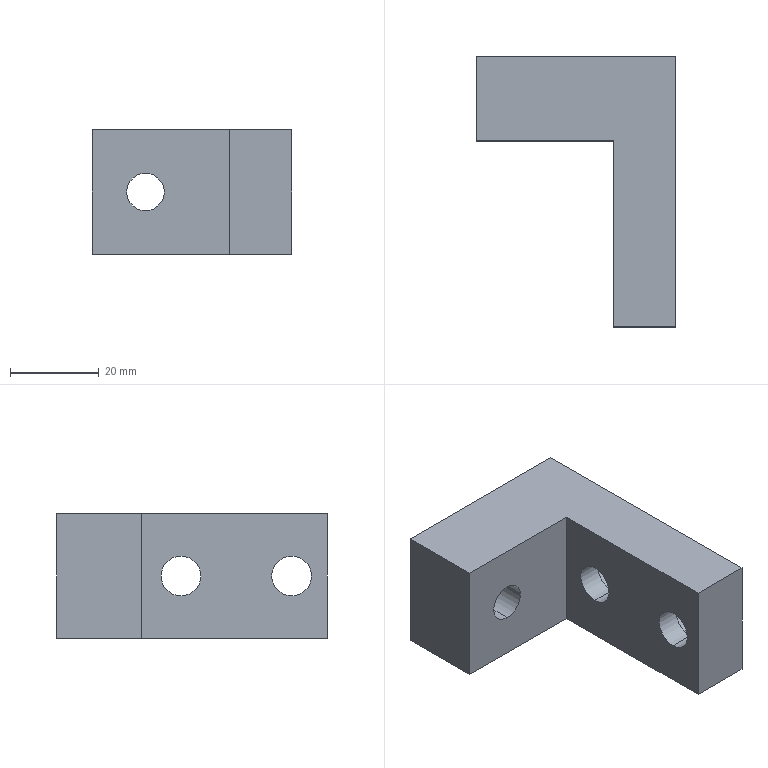Part | STEP file | PN_0002 (connecting block) | 1 solid | 20 faces | box 45 x 61 x 28 mm | volume 35599 mm3 | cylinder 10 | plane 10 | commonest cylinder face diameters 9 x4 15 x4 8.5 x2
STEP:
#1=CARTESIAN_POINT('',(0.,0.,0.));
#2=DIRECTION('',(0.,0.,1.));
#3=DIRECTION('',(1.,0.,0.));
#4=AXIS2_PLACEMENT_3D('',#1,#2,#3);
#5=CARTESIAN_POINT('',(-33.,42.,4.25));
#6=VERTEX_POINT('',#5);
#7=CARTESIAN_POINT('',(-33.,61.,4.25));
#8=VERTEX_POINT('',#7);
#9=CARTESIAN_POINT('',(-33.,61.,4.25));
#10=DIRECTION('',(0.,1.,0.));
#11=VECTOR('',#10,1.);
#12=LINE('',#9,#11);
#13=CARTESIAN_POINT('',(-33.,61.,0.));
#14=DIRECTION('',(0.,1.,0.));
#15=DIRECTION('',(0.,0.,1.));
#16=AXIS2_PLACEMENT_3D('',#13,#14,#15);
#17=CYLINDRICAL_SURFACE('',#16,4.25);
#18=CARTESIAN_POINT('',(6.283,0.));
#19=DIRECTION('',(0.,1.));
#20=VECTOR('',#19,1.);
#21=LINE('',#18,#20);
#22=(GEOMETRIC_REPRESENTATION_CONTEXT(2)PARAMETRIC_REPRESENTATION_CONTEXT()REPRESENTATION_CONTEXT('',''));
#23=DEFINITIONAL_REPRESENTATION('',(#21),#22);
#24=PCURVE('',#17,#23);
#25=CARTESIAN_POINT('',(-33.,61.,0.));
#26=DIRECTION('',(0.,1.,0.));
#27=DIRECTION('',(0.,0.,1.));
#28=AXIS2_PLACEMENT_3D('',#25,#26,#27);
#29=CYLINDRICAL_SURFACE('',#28,4.25);
#30=CARTESIAN_POINT('',(0.,0.));
#31=DIRECTION('',(0.,1.));
#32=VECTOR('',#31,1.);
#33=LINE('',#30,#32);
#34=(GEOMETRIC_REPRESENTATION_CONTEXT(2)PARAMETRIC_REPRESENTATION_CONTEXT()REPRESENTATION_CONTEXT('',''));
#35=DEFINITIONAL_REPRESENTATION('',(#33),#34);
#36=PCURVE('',#29,#35);
#37=SURFACE_CURVE('',#12,(#24,#36),.PCURVE_S1.);
#38=EDGE_CURVE('',#6,#8,#37,.T.);
#39=ORIENTED_EDGE('',*,*,#38,.T.);
#40=CARTESIAN_POINT('',(-33.,61.,-4.25));
#41=VERTEX_POINT('',#40);
#42=CARTESIAN_POINT('',(-33.,61.,0.));
#43=DIRECTION('',(0.,1.,0.));
#44=DIRECTION('',(0.,0.,1.));
#45=AXIS2_PLACEMENT_3D('',#42,#43,#44);
#46=CIRCLE('',#45,4.25);
#47=CARTESIAN_POINT('',(0.,0.));
#48=DIRECTION('',(1.,0.));
#49=VECTOR('',#48,1.);
#50=LINE('',#47,#49);
#51=(GEOMETRIC_REPRESENTATION_CONTEXT(2)PARAMETRIC_REPRESENTATION_CONTEXT()REPRESENTATION_CONTEXT('',''));
#52=DEFINITIONAL_REPRESENTATION('',(#50),#51);
#53=PCURVE('',#17,#52);
#54=CARTESIAN_POINT('',(0.,61.,14.));
#55=DIRECTION('',(0.,-1.,0.));
#56=DIRECTION('',(1.,0.,0.));
#57=AXIS2_PLACEMENT_3D('',#54,#55,#56);
#58=PLANE('',#57);
#59=CARTESIAN_POINT('',(-33.,-9.75));
#60=CARTESIAN_POINT('',(-25.639,-9.75));
#61=CARTESIAN_POINT('',(-29.319,-16.125));
#62=CARTESIAN_POINT('',(-33.,-22.5));
#63=CARTESIAN_POINT('',(-36.681,-16.125));
#64=CARTESIAN_POINT('',(-40.361,-9.75));
#65=CARTESIAN_POINT('',(-33.,-9.75));
#66=(BOUNDED_CURVE()B_SPLINE_CURVE(2,(#59,#60,#61,#62,#63,#64,#65),.UNSPECIFIED.,.T.,.F.)B_SPLINE_CURVE_WITH_KNOTS((1,2,2,2,2,1),(-2.094,0.,2.094,4.189,6.283,8.378),.UNSPECIFIED.)CURVE()GEOMETRIC_REPRESENTATION_ITEM()RATIONAL_B_SPLINE_CURVE((1.,0.5,1.,0.5,1.,0.5,1.))REPRESENTATION_ITEM(''));
#67=(GEOMETRIC_REPRESENTATION_CONTEXT(2)PARAMETRIC_REPRESENTATION_CONTEXT()REPRESENTATION_CONTEXT('',''));
#68=DEFINITIONAL_REPRESENTATION('',(#66),#67);
#69=PCURVE('',#58,#68);
#70=SURFACE_CURVE('',#46,(#53,#69),.PCURVE_S1.);
#71=EDGE_CURVE('',#41,#8,#70,.T.);
#72=ORIENTED_EDGE('',*,*,#71,.F.);
#73=CARTESIAN_POINT('',(-33.,42.,-4.25));
#74=VERTEX_POINT('',#73);
#75=CARTESIAN_POINT('',(-33.,61.,-4.25));
#76=DIRECTION('',(0.,1.,0.));
#77=VECTOR('',#76,1.);
#78=LINE('',#75,#77);
#79=CARTESIAN_POINT('',(3.142,0.));
#80=DIRECTION('',(0.,1.));
#81=VECTOR('',#80,1.);
#82=LINE('',#79,#81);
#83=(GEOMETRIC_REPRESENTATION_CONTEXT(2)PARAMETRIC_REPRESENTATION_CONTEXT()REPRESENTATION_CONTEXT('',''));
#84=DEFINITIONAL_REPRESENTATION('',(#82),#83);
#85=PCURVE('',#17,#84);
#86=CARTESIAN_POINT('',(3.142,0.));
#87=DIRECTION('',(0.,1.));
#88=VECTOR('',#87,1.);
#89=LINE('',#86,#88);
#90=(GEOMETRIC_REPRESENTATION_CONTEXT(2)PARAMETRIC_REPRESENTATION_CONTEXT()REPRESENTATION_CONTEXT('',''));
#91=DEFINITIONAL_REPRESENTATION('',(#89),#90);
#92=PCURVE('',#29,#91);
#93=SURFACE_CURVE('',#78,(#85,#92),.PCURVE_S1.);
#94=EDGE_CURVE('',#74,#41,#93,.T.);
#95=ORIENTED_EDGE('',*,*,#94,.F.);
#96=CARTESIAN_POINT('',(-33.,42.,0.));
#97=DIRECTION('',(0.,1.,0.));
#98=DIRECTION('',(-1.,0.,0.));
#99=AXIS2_PLACEMENT_3D('',#96,#97,#98);
#100=CIRCLE('',#99,4.25);
#101=CARTESIAN_POINT('',(-1.571,-19.));
#102=DIRECTION('',(1.,0.));
#103=VECTOR('',#102,1.);
#104=LINE('',#101,#103);
#105=(GEOMETRIC_REPRESENTATION_CONTEXT(2)PARAMETRIC_REPRESENTATION_CONTEXT()REPRESENTATION_CONTEXT('',''));
#106=DEFINITIONAL_REPRESENTATION('',(#104),#105);
#107=PCURVE('',#17,#106);
#108=CARTESIAN_POINT('',(-14.,42.,14.));
#109=DIRECTION('',(0.,1.,0.));
#110=DIRECTION('',(-1.,0.,0.));
#111=AXIS2_PLACEMENT_3D('',#108,#109,#110);
#112=PLANE('',#111);
#113=CARTESIAN_POINT('',(19.,-14.));
#114=DIRECTION('',(1.,0.));
#115=AXIS2_PLACEMENT_2D('',#113,#114);
#116=CIRCLE('',#115,4.25);
#117=(GEOMETRIC_REPRESENTATION_CONTEXT(2)PARAMETRIC_REPRESENTATION_CONTEXT()REPRESENTATION_CONTEXT('',''));
#118=DEFINITIONAL_REPRESENTATION('',(#116),#117);
#119=PCURVE('',#112,#118);
#120=SURFACE_CURVE('',#100,(#107,#119),.PCURVE_S1.);
#121=EDGE_CURVE('',#74,#6,#120,.T.);
#122=ORIENTED_EDGE('',*,*,#121,.T.);
#123=EDGE_LOOP('',(#39,#72,#95,#122));
#124=FACE_BOUND('',#123,.F.);
#125=ADVANCED_FACE('',(#124),#17,.F.);
#126=CARTESIAN_POINT('',(-8.6,33.,-7.5));
#127=VERTEX_POINT('',#126);
#128=CARTESIAN_POINT('',(0.,33.,-7.5));
#129=VERTEX_POINT('',#128);
#130=CARTESIAN_POINT('',(0.,33.,-7.5));
#131=DIRECTION('',(1.,0.,0.));
#132=VECTOR('',#131,1.);
#133=LINE('',#130,#132);
#134=CARTESIAN_POINT('',(0.,33.,0.));
#135=DIRECTION('',(1.,0.,0.));
#136=DIRECTION('',(0.,0.,-1.));
#137=AXIS2_PLACEMENT_3D('',#134,#135,#136);
#138=CYLINDRICAL_SURFACE('',#137,7.5);
#139=CARTESIAN_POINT('',(6.283,0.));
#140=DIRECTION('',(0.,1.));
#141=VECTOR('',#140,1.);
#142=LINE('',#139,#141);
#143=(GEOMETRIC_REPRESENTATION_CONTEXT(2)PARAMETRIC_REPRESENTATION_CONTEXT()REPRESENTATION_CONTEXT('',''));
#144=DEFINITIONAL_REPRESENTATION('',(#142),#143);
#145=PCURVE('',#138,#144);
#146=CARTESIAN_POINT('',(0.,33.,0.));
#147=DIRECTION('',(1.,0.,0.));
#148=DIRECTION('',(0.,0.,-1.));
#149=AXIS2_PLACEMENT_3D('',#146,#147,#148);
#150=CYLINDRICAL_SURFACE('',#149,7.5);
#151=CARTESIAN_POINT('',(0.,0.));
#152=DIRECTION('',(0.,1.));
#153=VECTOR('',#152,1.);
#154=LINE('',#151,#153);
#155=(GEOMETRIC_REPRESENTATION_CONTEXT(2)PARAMETRIC_REPRESENTATION_CONTEXT()REPRESENTATION_CONTEXT('',''));
#156=DEFINITIONAL_REPRESENTATION('',(#154),#155);
#157=PCURVE('',#150,#156);
#158=SURFACE_CURVE('',#133,(#145,#157),.PCURVE_S1.);
#159=EDGE_CURVE('',#127,#129,#158,.T.);
#160=ORIENTED_EDGE('',*,*,#159,.T.);
#161=CARTESIAN_POINT('',(0.,33.,7.5));
#162=VERTEX_POINT('',#161);
#163=CARTESIAN_POINT('',(0.,33.,0.));
#164=DIRECTION('',(1.,0.,0.));
#165=DIRECTION('',(0.,0.,-1.));
#166=AXIS2_PLACEMENT_3D('',#163,#164,#165);
#167=CIRCLE('',#166,7.5);
#168=CARTESIAN_POINT('',(0.,0.));
#169=DIRECTION('',(1.,0.));
#170=VECTOR('',#169,1.);
#171=LINE('',#168,#170);
#172=(GEOMETRIC_REPRESENTATION_CONTEXT(2)PARAMETRIC_REPRESENTATION_CONTEXT()REPRESENTATION_CONTEXT('',''));
#173=DEFINITIONAL_REPRESENTATION('',(#171),#172);
#174=PCURVE('',#138,#173);
#175=CARTESIAN_POINT('',(0.,0.,14.));
#176=DIRECTION('',(-1.,0.,0.));
#177=DIRECTION('',(0.,0.,1.));
#178=AXIS2_PLACEMENT_3D('',#175,#176,#177);
#179=PLANE('',#178);
#180=CARTESIAN_POINT('',(-21.5,33.));
#181=CARTESIAN_POINT('',(-21.5,45.99));
#182=CARTESIAN_POINT('',(-10.25,39.495));
#183=CARTESIAN_POINT('',(1.,33.));
#184=CARTESIAN_POINT('',(-10.25,26.505));
#185=CARTESIAN_POINT('',(-21.5,20.01));
#186=CARTESIAN_POINT('',(-21.5,33.));
#187=(BOUNDED_CURVE()B_SPLINE_CURVE(2,(#180,#181,#182,#183,#184,#185,#186),.UNSPECIFIED.,.T.,.F.)B_SPLINE_CURVE_WITH_KNOTS((1,2,2,2,2,1),(-2.094,0.,2.094,4.189,6.283,8.378),.UNSPECIFIED.)CURVE()GEOMETRIC_REPRESENTATION_ITEM()RATIONAL_B_SPLINE_CURVE((1.,0.5,1.,0.5,1.,0.5,1.))REPRESENTATION_ITEM(''));
#188=(GEOMETRIC_REPRESENTATION_CONTEXT(2)PARAMETRIC_REPRESENTATION_CONTEXT()REPRESENTATION_CONTEXT('',''));
#189=DEFINITIONAL_REPRESENTATION('',(#187),#188);
#190=PCURVE('',#179,#189);
#191=SURFACE_CURVE('',#167,(#174,#190),.PCURVE_S1.);
#192=EDGE_CURVE('',#162,#129,#191,.T.);
#193=ORIENTED_EDGE('',*,*,#192,.F.);
#194=CARTESIAN_POINT('',(-8.6,33.,7.5));
#195=VERTEX_POINT('',#194);
#196=CARTESIAN_POINT('',(0.,33.,7.5));
#197=DIRECTION('',(1.,0.,0.));
#198=VECTOR('',#197,1.);
#199=LINE('',#196,#198);
#200=CARTESIAN_POINT('',(3.142,0.));
#201=DIRECTION('',(0.,1.));
#202=VECTOR('',#201,1.);
#203=LINE('',#200,#202);
#204=(GEOMETRIC_REPRESENTATION_CONTEXT(2)PARAMETRIC_REPRESENTATION_CONTEXT()REPRESENTATION_CONTEXT('',''));
#205=DEFINITIONAL_REPRESENTATION('',(#203),#204);
#206=PCURVE('',#138,#205);
#207=CARTESIAN_POINT('',(3.142,0.));
#208=DIRECTION('',(0.,1.));
#209=VECTOR('',#208,1.);
#210=LINE('',#207,#209);
#211=(GEOMETRIC_REPRESENTATION_CONTEXT(2)PARAMETRIC_REPRESENTATION_CONTEXT()REPRESENTATION_CONTEXT('',''));
#212=DEFINITIONAL_REPRESENTATION('',(#210),#211);
#213=PCURVE('',#150,#212);
#214=SURFACE_CURVE('',#199,(#206,#213),.PCURVE_S1.);
#215=EDGE_CURVE('',#195,#162,#214,.T.);
#216=ORIENTED_EDGE('',*,*,#215,.F.);
#217=CARTESIAN_POINT('',(-8.6,33.,0.));
#218=DIRECTION('',(1.,0.,0.));
#219=DIRECTION('',(0.,0.,-1.));
#220=AXIS2_PLACEMENT_3D('',#217,#218,#219);
#221=CIRCLE('',#220,7.5);
#222=CARTESIAN_POINT('',(0.,-8.6));
#223=DIRECTION('',(1.,0.));
#224=VECTOR('',#223,1.);
#225=LINE('',#222,#224);
#226=(GEOMETRIC_REPRESENTATION_CONTEXT(2)PARAMETRIC_REPRESENTATION_CONTEXT()REPRESENTATION_CONTEXT('',''));
#227=DEFINITIONAL_REPRESENTATION('',(#225),#226);
#228=PCURVE('',#138,#227);
#229=CARTESIAN_POINT('',(-8.6,37.5,0.));
#230=DIRECTION('',(-1.,0.,0.));
#231=DIRECTION('',(0.,0.,1.));
#232=AXIS2_PLACEMENT_3D('',#229,#230,#231);
#233=PLANE('',#232);
#234=CARTESIAN_POINT('',(-7.5,-4.5));
#235=CARTESIAN_POINT('',(-7.5,8.49));
#236=CARTESIAN_POINT('',(3.75,1.995));
#237=CARTESIAN_POINT('',(15.,-4.5));
#238=CARTESIAN_POINT('',(3.75,-10.995));
#239=CARTESIAN_POINT('',(-7.5,-17.49));
#240=CARTESIAN_POINT('',(-7.5,-4.5));
#241=(BOUNDED_CURVE()B_SPLINE_CURVE(2,(#234,#235,#236,#237,#238,#239,#240),.UNSPECIFIED.,.T.,.F.)B_SPLINE_CURVE_WITH_KNOTS((1,2,2,2,2,1),(-2.094,0.,2.094,4.189,6.283,8.378),.UNSPECIFIED.)CURVE()GEOMETRIC_REPRESENTATION_ITEM()RATIONAL_B_SPLINE_CURVE((1.,0.5,1.,0.5,1.,0.5,1.))REPRESENTATION_ITEM(''));
#242=(GEOMETRIC_REPRESENTATION_CONTEXT(2)PARAMETRIC_REPRESENTATION_CONTEXT()REPRESENTATION_CONTEXT('',''));
#243=DEFINITIONAL_REPRESENTATION('',(#241),#242);
#244=PCURVE('',#233,#243);
#245=SURFACE_CURVE('',#221,(#228,#244),.PCURVE_S1.);
#246=EDGE_CURVE('',#195,#127,#245,.T.);
#247=ORIENTED_EDGE('',*,*,#246,.T.);
#248=EDGE_LOOP('',(#160,#193,#216,#247));
#249=FACE_BOUND('',#248,.F.);
#250=ADVANCED_FACE('',(#249),#138,.F.);
#251=CARTESIAN_POINT('',(-14.,33.,-4.5));
#252=VERTEX_POINT('',#251);
#253=CARTESIAN_POINT('',(-8.6,33.,-4.5));
#254=VERTEX_POINT('',#253);
#255=CARTESIAN_POINT('',(0.,33.,-4.5));
#256=DIRECTION('',(1.,0.,0.));
#257=VECTOR('',#256,1.);
#258=LINE('',#255,#257);
#259=CARTESIAN_POINT('',(0.,33.,0.));
#260=DIRECTION('',(1.,0.,0.));
#261=DIRECTION('',(0.,0.,-1.));
#262=AXIS2_PLACEMENT_3D('',#259,#260,#261);
#263=CYLINDRICAL_SURFACE('',#262,4.5);
#264=CARTESIAN_POINT('',(6.283,0.));
#265=DIRECTION('',(0.,1.));
#266=VECTOR('',#265,1.);
#267=LINE('',#264,#266);
#268=(GEOMETRIC_REPRESENTATION_CONTEXT(2)PARAMETRIC_REPRESENTATION_CONTEXT()REPRESENTATION_CONTEXT('',''));
#269=DEFINITIONAL_REPRESENTATION('',(#267),#268);
#270=PCURVE('',#263,#269);
#271=CARTESIAN_POINT('',(0.,33.,0.));
#272=DIRECTION('',(1.,0.,0.));
#273=DIRECTION('',(0.,0.,-1.));
#274=AXIS2_PLACEMENT_3D('',#271,#272,#273);
#275=CYLINDRICAL_SURFACE('',#274,4.5);
#276=CARTESIAN_POINT('',(0.,0.));
#277=DIRECTION('',(0.,1.));
#278=VECTOR('',#277,1.);
#279=LINE('',#276,#278);
#280=(GEOMETRIC_REPRESENTATION_CONTEXT(2)PARAMETRIC_REPRESENTATION_CONTEXT()REPRESENTATION_CONTEXT('',''));
#281=DEFINITIONAL_REPRESENTATION('',(#279),#280);
#282=PCURVE('',#275,#281);
#283=SURFACE_CURVE('',#258,(#270,#282),.PCURVE_S1.);
#284=EDGE_CURVE('',#252,#254,#283,.T.);
#285=ORIENTED_EDGE('',*,*,#284,.T.);
#286=CARTESIAN_POINT('',(-8.6,33.,4.5));
#287=VERTEX_POINT('',#286);
#288=CARTESIAN_POINT('',(-8.6,33.,0.));
#289=DIRECTION('',(1.,0.,0.));
#290=DIRECTION('',(0.,0.,-1.));
#291=AXIS2_PLACEMENT_3D('',#288,#289,#290);
#292=CIRCLE('',#291,4.5);
#293=CARTESIAN_POINT('',(0.,-8.6));
#294=DIRECTION('',(1.,0.));
#295=VECTOR('',#294,1.);
#296=LINE('',#293,#295);
#297=(GEOMETRIC_REPRESENTATION_CONTEXT(2)PARAMETRIC_REPRESENTATION_CONTEXT()REPRESENTATION_CONTEXT('',''));
#298=DEFINITIONAL_REPRESENTATION('',(#296),#297);
#299=PCURVE('',#263,#298);
#300=CARTESIAN_POINT('',(-4.5,-4.5));
#301=CARTESIAN_POINT('',(-4.5,3.294));
#302=CARTESIAN_POINT('',(2.25,-0.6029));
#303=CARTESIAN_POINT('',(9.,-4.5));
#304=CARTESIAN_POINT('',(2.25,-8.397));
#305=CARTESIAN_POINT('',(-4.5,-12.294));
#306=CARTESIAN_POINT('',(-4.5,-4.5));
#307=(BOUNDED_CURVE()B_SPLINE_CURVE(2,(#300,#301,#302,#303,#304,#305,#306),.UNSPECIFIED.,.T.,.F.)B_SPLINE_CURVE_WITH_KNOTS((1,2,2,2,2,1),(-2.094,0.,2.094,4.189,6.283,8.378),.UNSPECIFIED.)CURVE()GEOMETRIC_REPRESENTATION_ITEM()RATIONAL_B_SPLINE_CURVE((1.,0.5,1.,0.5,1.,0.5,1.))REPRESENTATION_ITEM(''));
#308=(GEOMETRIC_REPRESENTATION_CONTEXT(2)PARAMETRIC_REPRESENTATION_CONTEXT()REPRESENTATION_CONTEXT('',''));
#309=DEFINITIONAL_REPRESENTATION('',(#307),#308);
#310=PCURVE('',#233,#309);
#311=SURFACE_CURVE('',#292,(#299,#310),.PCURVE_S1.);
#312=EDGE_CURVE('',#287,#254,#311,.T.);
#313=ORIENTED_EDGE('',*,*,#312,.F.);
#314=CARTESIAN_POINT('',(-14.,33.,4.5));
#315=VERTEX_POINT('',#314);
#316=CARTESIAN_POINT('',(0.,33.,4.5));
#317=DIRECTION('',(1.,0.,0.));
#318=VECTOR('',#317,1.);
#319=LINE('',#316,#318);
#320=CARTESIAN_POINT('',(3.142,0.));
#321=DIRECTION('',(0.,1.));
#322=VECTOR('',#321,1.);
#323=LINE('',#320,#322);
#324=(GEOMETRIC_REPRESENTATION_CONTEXT(2)PARAMETRIC_REPRESENTATION_CONTEXT()REPRESENTATION_CONTEXT('',''));
#325=DEFINITIONAL_REPRESENTATION('',(#323),#324);
#326=PCURVE('',#263,#325);
#327=CARTESIAN_POINT('',(3.142,0.));
#328=DIRECTION('',(0.,1.));
#329=VECTOR('',#328,1.);
#330=LINE('',#327,#329);
#331=(GEOMETRIC_REPRESENTATION_CONTEXT(2)PARAMETRIC_REPRESENTATION_CONTEXT()REPRESENTATION_CONTEXT('',''));
#332=DEFINITIONAL_REPRESENTATION('',(#330),#331);
#333=PCURVE('',#275,#332);
#334=SURFACE_CURVE('',#319,(#326,#333),.PCURVE_S1.);
#335=EDGE_CURVE('',#315,#287,#334,.T.);
#336=ORIENTED_EDGE('',*,*,#335,.F.);
#337=CARTESIAN_POINT('',(-14.,33.,0.));
#338=DIRECTION('',(1.,0.,0.));
#339=DIRECTION('',(0.,0.,-1.));
#340=AXIS2_PLACEMENT_3D('',#337,#338,#339);
#341=CIRCLE('',#340,4.5);
#342=CARTESIAN_POINT('',(0.,-14.));
#343=DIRECTION('',(1.,0.));
#344=VECTOR('',#343,1.);
#345=LINE('',#342,#344);
#346=(GEOMETRIC_REPRESENTATION_CONTEXT(2)PARAMETRIC_REPRESENTATION_CONTEXT()REPRESENTATION_CONTEXT('',''));
#347=DEFINITIONAL_REPRESENTATION('',(#345),#346);
#348=PCURVE('',#263,#347);
#349=CARTESIAN_POINT('',(-14.,0.,14.));
#350=DIRECTION('',(1.,0.,0.));
#351=DIRECTION('',(0.,0.,-1.));
#352=AXIS2_PLACEMENT_3D('',#349,#350,#351);
#353=PLANE('',#352);
#354=CARTESIAN_POINT('',(14.,33.));
#355=DIRECTION('',(1.,0.));
#356=AXIS2_PLACEMENT_2D('',#354,#355);
#357=CIRCLE('',#356,4.5);
#358=(GEOMETRIC_REPRESENTATION_CONTEXT(2)PARAMETRIC_REPRESENTATION_CONTEXT()REPRESENTATION_CONTEXT('',''));
#359=DEFINITIONAL_REPRESENTATION('',(#357),#358);
#360=PCURVE('',#353,#359);
#361=SURFACE_CURVE('',#341,(#348,#360),.PCURVE_S1.);
#362=EDGE_CURVE('',#315,#252,#361,.T.);
#363=ORIENTED_EDGE('',*,*,#362,.T.);
#364=EDGE_LOOP('',(#285,#313,#336,#363));
#365=FACE_BOUND('',#364,.F.);
#366=ADVANCED_FACE('',(#365),#263,.F.);
#367=CARTESIAN_POINT('',(-8.6,8.,-7.5));
#368=VERTEX_POINT('',#367);
#369=CARTESIAN_POINT('',(0.,8.,-7.5));
#370=VERTEX_POINT('',#369);
#371=CARTESIAN_POINT('',(0.,8.,-7.5));
#372=DIRECTION('',(1.,0.,0.));
#373=VECTOR('',#372,1.);
#374=LINE('',#371,#373);
#375=CARTESIAN_POINT('',(0.,8.,0.));
#376=DIRECTION('',(1.,0.,0.));
#377=DIRECTION('',(0.,0.,-1.));
#378=AXIS2_PLACEMENT_3D('',#375,#376,#377);
#379=CYLINDRICAL_SURFACE('',#378,7.5);
#380=CARTESIAN_POINT('',(6.283,0.));
#381=DIRECTION('',(0.,1.));
#382=VECTOR('',#381,1.);
#383=LINE('',#380,#382);
#384=(GEOMETRIC_REPRESENTATION_CONTEXT(2)PARAMETRIC_REPRESENTATION_CONTEXT()REPRESENTATION_CONTEXT('',''));
#385=DEFINITIONAL_REPRESENTATION('',(#383),#384);
#386=PCURVE('',#379,#385);
#387=CARTESIAN_POINT('',(0.,8.,0.));
#388=DIRECTION('',(1.,0.,0.));
#389=DIRECTION('',(0.,0.,-1.));
#390=AXIS2_PLACEMENT_3D('',#387,#388,#389);
#391=CYLINDRICAL_SURFACE('',#390,7.5);
#392=CARTESIAN_POINT('',(0.,0.));
#393=DIRECTION('',(0.,1.));
#394=VECTOR('',#393,1.);
#395=LINE('',#392,#394);
#396=(GEOMETRIC_REPRESENTATION_CONTEXT(2)PARAMETRIC_REPRESENTATION_CONTEXT()REPRESENTATION_CONTEXT('',''));
#397=DEFINITIONAL_REPRESENTATION('',(#395),#396);
#398=PCURVE('',#391,#397);
#399=SURFACE_CURVE('',#374,(#386,#398),.PCURVE_S1.);
#400=EDGE_CURVE('',#368,#370,#399,.T.);
#401=ORIENTED_EDGE('',*,*,#400,.T.);
#402=CARTESIAN_POINT('',(0.,8.,7.5));
#403=VERTEX_POINT('',#402);
#404=CARTESIAN_POINT('',(0.,8.,0.));
#405=DIRECTION('',(1.,0.,0.));
#406=DIRECTION('',(0.,0.,-1.));
#407=AXIS2_PLACEMENT_3D('',#404,#405,#406);
#408=CIRCLE('',#407,7.5);
#409=CARTESIAN_POINT('',(0.,0.));
#410=DIRECTION('',(1.,0.));
#411=VECTOR('',#410,1.);
#412=LINE('',#409,#411);
#413=(GEOMETRIC_REPRESENTATION_CONTEXT(2)PARAMETRIC_REPRESENTATION_CONTEXT()REPRESENTATION_CONTEXT('',''));
#414=DEFINITIONAL_REPRESENTATION('',(#412),#413);
#415=PCURVE('',#379,#414);
#416=CARTESIAN_POINT('',(-21.5,8.));
#417=CARTESIAN_POINT('',(-21.5,20.99));
#418=CARTESIAN_POINT('',(-10.25,14.495));
#419=CARTESIAN_POINT('',(1.,8.));
#420=CARTESIAN_POINT('',(-10.25,1.505));
#421=CARTESIAN_POINT('',(-21.5,-4.99));
#422=CARTESIAN_POINT('',(-21.5,8.));
#423=(BOUNDED_CURVE()B_SPLINE_CURVE(2,(#416,#417,#418,#419,#420,#421,#422),.UNSPECIFIED.,.T.,.F.)B_SPLINE_CURVE_WITH_KNOTS((1,2,2,2,2,1),(-2.094,0.,2.094,4.189,6.283,8.378),.UNSPECIFIED.)CURVE()GEOMETRIC_REPRESENTATION_ITEM()RATIONAL_B_SPLINE_CURVE((1.,0.5,1.,0.5,1.,0.5,1.))REPRESENTATION_ITEM(''));
#424=(GEOMETRIC_REPRESENTATION_CONTEXT(2)PARAMETRIC_REPRESENTATION_CONTEXT()REPRESENTATION_CONTEXT('',''));
#425=DEFINITIONAL_REPRESENTATION('',(#423),#424);
#426=PCURVE('',#179,#425);
#427=SURFACE_CURVE('',#408,(#415,#426),.PCURVE_S1.);
#428=EDGE_CURVE('',#403,#370,#427,.T.);
#429=ORIENTED_EDGE('',*,*,#428,.F.);
#430=CARTESIAN_POINT('',(-8.6,8.,7.5));
#431=VERTEX_POINT('',#430);
#432=CARTESIAN_POINT('',(0.,8.,7.5));
#433=DIRECTION('',(1.,0.,0.));
#434=VECTOR('',#433,1.);
#435=LINE('',#432,#434);
#436=CARTESIAN_POINT('',(3.142,0.));
#437=DIRECTION('',(0.,1.));
#438=VECTOR('',#437,1.);
#439=LINE('',#436,#438);
#440=(GEOMETRIC_REPRESENTATION_CONTEXT(2)PARAMETRIC_REPRESENTATION_CONTEXT()REPRESENTATION_CONTEXT('',''));
#441=DEFINITIONAL_REPRESENTATION('',(#439),#440);
#442=PCURVE('',#379,#441);
#443=CARTESIAN_POINT('',(3.142,0.));
#444=DIRECTION('',(0.,1.));
#445=VECTOR('',#444,1.);
#446=LINE('',#443,#445);
#447=(GEOMETRIC_REPRESENTATION_CONTEXT(2)PARAMETRIC_REPRESENTATION_CONTEXT()REPRESENTATION_CONTEXT('',''));
#448=DEFINITIONAL_REPRESENTATION('',(#446),#447);
#449=PCURVE('',#391,#448);
#450=SURFACE_CURVE('',#435,(#442,#449),.PCURVE_S1.);
#451=EDGE_CURVE('',#431,#403,#450,.T.);
#452=ORIENTED_EDGE('',*,*,#451,.F.);
#453=CARTESIAN_POINT('',(-8.6,8.,0.));
#454=DIRECTION('',(1.,0.,0.));
#455=DIRECTION('',(0.,0.,-1.));
#456=AXIS2_PLACEMENT_3D('',#453,#454,#455);
#457=CIRCLE('',#456,7.5);
#458=CARTESIAN_POINT('',(0.,-8.6));
#459=DIRECTION('',(1.,0.));
#460=VECTOR('',#459,1.);
#461=LINE('',#458,#460);
#462=(GEOMETRIC_REPRESENTATION_CONTEXT(2)PARAMETRIC_REPRESENTATION_CONTEXT()REPRESENTATION_CONTEXT('',''));
#463=DEFINITIONAL_REPRESENTATION('',(#461),#462);
#464=PCURVE('',#379,#463);
#465=CARTESIAN_POINT('',(-8.6,12.5,0.));
#466=DIRECTION('',(-1.,0.,0.));
#467=DIRECTION('',(0.,0.,1.));
#468=AXIS2_PLACEMENT_3D('',#465,#466,#467);
#469=PLANE('',#468);
#470=CARTESIAN_POINT('',(-7.5,-4.5));
#471=CARTESIAN_POINT('',(-7.5,8.49));
#472=CARTESIAN_POINT('',(3.75,1.995));
#473=CARTESIAN_POINT('',(15.,-4.5));
#474=CARTESIAN_POINT('',(3.75,-10.995));
#475=CARTESIAN_POINT('',(-7.5,-17.49));
#476=CARTESIAN_POINT('',(-7.5,-4.5));
#477=(BOUNDED_CURVE()B_SPLINE_CURVE(2,(#470,#471,#472,#473,#474,#475,#476),.UNSPECIFIED.,.T.,.F.)B_SPLINE_CURVE_WITH_KNOTS((1,2,2,2,2,1),(-2.094,0.,2.094,4.189,6.283,8.378),.UNSPECIFIED.)CURVE()GEOMETRIC_REPRESENTATION_ITEM()RATIONAL_B_SPLINE_CURVE((1.,0.5,1.,0.5,1.,0.5,1.))REPRESENTATION_ITEM(''));
#478=(GEOMETRIC_REPRESENTATION_CONTEXT(2)PARAMETRIC_REPRESENTATION_CONTEXT()REPRESENTATION_CONTEXT('',''));
#479=DEFINITIONAL_REPRESENTATION('',(#477),#478);
#480=PCURVE('',#469,#479);
#481=SURFACE_CURVE('',#457,(#464,#480),.PCURVE_S1.);
#482=EDGE_CURVE('',#431,#368,#481,.T.);
#483=ORIENTED_EDGE('',*,*,#482,.T.);
#484=EDGE_LOOP('',(#401,#429,#452,#483));
#485=FACE_BOUND('',#484,.F.);
#486=ADVANCED_FACE('',(#485),#379,.F.);
#487=CARTESIAN_POINT('',(-14.,8.,-4.5));
#488=VERTEX_POINT('',#487);
#489=CARTESIAN_POINT('',(-8.6,8.,-4.5));
#490=VERTEX_POINT('',#489);
#491=CARTESIAN_POINT('',(0.,8.,-4.5));
#492=DIRECTION('',(1.,0.,0.));
#493=VECTOR('',#492,1.);
#494=LINE('',#491,#493);
#495=CARTESIAN_POINT('',(0.,8.,0.));
#496=DIRECTION('',(1.,0.,0.));
#497=DIRECTION('',(0.,0.,-1.));
#498=AXIS2_PLACEMENT_3D('',#495,#496,#497);
#499=CYLINDRICAL_SURFACE('',#498,4.5);
#500=CARTESIAN_POINT('',(6.283,0.));
#501=DIRECTION('',(0.,1.));
#502=VECTOR('',#501,1.);
#503=LINE('',#500,#502);
#504=(GEOMETRIC_REPRESENTATION_CONTEXT(2)PARAMETRIC_REPRESENTATION_CONTEXT()REPRESENTATION_CONTEXT('',''));
#505=DEFINITIONAL_REPRESENTATION('',(#503),#504);
#506=PCURVE('',#499,#505);
#507=CARTESIAN_POINT('',(0.,8.,0.));
#508=DIRECTION('',(1.,0.,0.));
#509=DIRECTION('',(0.,0.,-1.));
#510=AXIS2_PLACEMENT_3D('',#507,#508,#509);
#511=CYLINDRICAL_SURFACE('',#510,4.5);
#512=CARTESIAN_POINT('',(0.,0.));
#513=DIRECTION('',(0.,1.));
#514=VECTOR('',#513,1.);
#515=LINE('',#512,#514);
#516=(GEOMETRIC_REPRESENTATION_CONTEXT(2)PARAMETRIC_REPRESENTATION_CONTEXT()REPRESENTATION_CONTEXT('',''));
#517=DEFINITIONAL_REPRESENTATION('',(#515),#516);
#518=PCURVE('',#511,#517);
#519=SURFACE_CURVE('',#494,(#506,#518),.PCURVE_S1.);
#520=EDGE_CURVE('',#488,#490,#519,.T.);
#521=ORIENTED_EDGE('',*,*,#520,.T.);
#522=CARTESIAN_POINT('',(-8.6,8.,4.5));
#523=VERTEX_POINT('',#522);
#524=CARTESIAN_POINT('',(-8.6,8.,0.));
#525=DIRECTION('',(1.,0.,0.));
#526=DIRECTION('',(0.,0.,-1.));
#527=AXIS2_PLACEMENT_3D('',#524,#525,#526);
#528=CIRCLE('',#527,4.5);
#529=CARTESIAN_POINT('',(0.,-8.6));
#530=DIRECTION('',(1.,0.));
#531=VECTOR('',#530,1.);
#532=LINE('',#529,#531);
#533=(GEOMETRIC_REPRESENTATION_CONTEXT(2)PARAMETRIC_REPRESENTATION_CONTEXT()REPRESENTATION_CONTEXT('',''));
#534=DEFINITIONAL_REPRESENTATION('',(#532),#533);
#535=PCURVE('',#499,#534);
#536=CARTESIAN_POINT('',(-4.5,-4.5));
#537=CARTESIAN_POINT('',(-4.5,3.294));
#538=CARTESIAN_POINT('',(2.25,-0.6029));
#539=CARTESIAN_POINT('',(9.,-4.5));
#540=CARTESIAN_POINT('',(2.25,-8.397));
#541=CARTESIAN_POINT('',(-4.5,-12.294));
#542=CARTESIAN_POINT('',(-4.5,-4.5));
#543=(BOUNDED_CURVE()B_SPLINE_CURVE(2,(#536,#537,#538,#539,#540,#541,#542),.UNSPECIFIED.,.T.,.F.)B_SPLINE_CURVE_WITH_KNOTS((1,2,2,2,2,1),(-2.094,0.,2.094,4.189,6.283,8.378),.UNSPECIFIED.)CURVE()GEOMETRIC_REPRESENTATION_ITEM()RATIONAL_B_SPLINE_CURVE((1.,0.5,1.,0.5,1.,0.5,1.))REPRESENTATION_ITEM(''));
#544=(GEOMETRIC_REPRESENTATION_CONTEXT(2)PARAMETRIC_REPRESENTATION_CONTEXT()REPRESENTATION_CONTEXT('',''));
#545=DEFINITIONAL_REPRESENTATION('',(#543),#544);
#546=PCURVE('',#469,#545);
#547=SURFACE_CURVE('',#528,(#535,#546),.PCURVE_S1.);
#548=EDGE_CURVE('',#523,#490,#547,.T.);
#549=ORIENTED_EDGE('',*,*,#548,.F.);
#550=CARTESIAN_POINT('',(-14.,8.,4.5));
#551=VERTEX_POINT('',#550);
#552=CARTESIAN_POINT('',(0.,8.,4.5));
#553=DIRECTION('',(1.,0.,0.));
#554=VECTOR('',#553,1.);
#555=LINE('',#552,#554);
#556=CARTESIAN_POINT('',(3.142,0.));
#557=DIRECTION('',(0.,1.));
#558=VECTOR('',#557,1.);
#559=LINE('',#556,#558);
#560=(GEOMETRIC_REPRESENTATION_CONTEXT(2)PARAMETRIC_REPRESENTATION_CONTEXT()REPRESENTATION_CONTEXT('',''));
#561=DEFINITIONAL_REPRESENTATION('',(#559),#560);
#562=PCURVE('',#499,#561);
#563=CARTESIAN_POINT('',(3.142,0.));
#564=DIRECTION('',(0.,1.));
#565=VECTOR('',#564,1.);
#566=LINE('',#563,#565);
#567=(GEOMETRIC_REPRESENTATION_CONTEXT(2)PARAMETRIC_REPRESENTATION_CONTEXT()REPRESENTATION_CONTEXT('',''));
#568=DEFINITIONAL_REPRESENTATION('',(#566),#567);
#569=PCURVE('',#511,#568);
#570=SURFACE_CURVE('',#555,(#562,#569),.PCURVE_S1.);
#571=EDGE_CURVE('',#551,#523,#570,.T.);
#572=ORIENTED_EDGE('',*,*,#571,.F.);
#573=CARTESIAN_POINT('',(-14.,8.,0.));
#574=DIRECTION('',(1.,0.,0.));
#575=DIRECTION('',(0.,0.,-1.));
#576=AXIS2_PLACEMENT_3D('',#573,#574,#575);
#577=CIRCLE('',#576,4.5);
#578=CARTESIAN_POINT('',(0.,-14.));
#579=DIRECTION('',(1.,0.));
#580=VECTOR('',#579,1.);
#581=LINE('',#578,#580);
#582=(GEOMETRIC_REPRESENTATION_CONTEXT(2)PARAMETRIC_REPRESENTATION_CONTEXT()REPRESENTATION_CONTEXT('',''));
#583=DEFINITIONAL_REPRESENTATION('',(#581),#582);
#584=PCURVE('',#499,#583);
#585=CARTESIAN_POINT('',(14.,8.));
#586=DIRECTION('',(1.,0.));
#587=AXIS2_PLACEMENT_2D('',#585,#586);
#588=CIRCLE('',#587,4.5);
#589=(GEOMETRIC_REPRESENTATION_CONTEXT(2)PARAMETRIC_REPRESENTATION_CONTEXT()REPRESENTATION_CONTEXT('',''));
#590=DEFINITIONAL_REPRESENTATION('',(#588),#589);
#591=PCURVE('',#353,#590);
#592=SURFACE_CURVE('',#577,(#584,#591),.PCURVE_S1.);
#593=EDGE_CURVE('',#551,#488,#592,.T.);
#594=ORIENTED_EDGE('',*,*,#593,.T.);
#595=EDGE_LOOP('',(#521,#549,#572,#594));
#596=FACE_BOUND('',#595,.F.);
#597=ADVANCED_FACE('',(#596),#499,.F.);
#598=CARTESIAN_POINT('',(-14.,0.,-14.));
#599=VERTEX_POINT('',#598);
#600=CARTESIAN_POINT('',(0.,0.,-14.));
#601=VERTEX_POINT('',#600);
#602=CARTESIAN_POINT('',(0.,0.,-14.));
#603=DIRECTION('',(1.,0.,0.));
#604=VECTOR('',#603,1.);
#605=LINE('',#602,#604);
#606=CARTESIAN_POINT('',(0.,0.,14.));
#607=DIRECTION('',(0.,1.,0.));
#608=DIRECTION('',(-1.,0.,0.));
#609=AXIS2_PLACEMENT_3D('',#606,#607,#608);
#610=PLANE('',#609);
#611=CARTESIAN_POINT('',(0.,-28.));
#612=DIRECTION('',(-1.,0.));
#613=VECTOR('',#612,1.);
#614=LINE('',#611,#613);
#615=(GEOMETRIC_REPRESENTATION_CONTEXT(2)PARAMETRIC_REPRESENTATION_CONTEXT()REPRESENTATION_CONTEXT('',''));
#616=DEFINITIONAL_REPRESENTATION('',(#614),#615);
#617=PCURVE('',#610,#616);
#618=CARTESIAN_POINT('',(0.,0.,-14.));
#619=DIRECTION('',(0.,0.,-1.));
#620=DIRECTION('',(-1.,0.,0.));
#621=AXIS2_PLACEMENT_3D('',#618,#619,#620);
#622=PLANE('',#621);
#623=CARTESIAN_POINT('',(0.,0.));
#624=DIRECTION('',(-1.,0.));
#625=VECTOR('',#624,1.);
#626=LINE('',#623,#625);
#627=(GEOMETRIC_REPRESENTATION_CONTEXT(2)PARAMETRIC_REPRESENTATION_CONTEXT()REPRESENTATION_CONTEXT('',''));
#628=DEFINITIONAL_REPRESENTATION('',(#626),#627);
#629=PCURVE('',#622,#628);
#630=SURFACE_CURVE('',#605,(#617,#629),.PCURVE_S1.);
#631=EDGE_CURVE('',#599,#601,#630,.T.);
#632=ORIENTED_EDGE('',*,*,#631,.T.);
#633=CARTESIAN_POINT('',(0.,0.,14.));
#634=VERTEX_POINT('',#633);
#635=CARTESIAN_POINT('',(0.,0.,14.));
#636=DIRECTION('',(0.,0.,-1.));
#637=VECTOR('',#636,1.);
#638=LINE('',#635,#637);
#639=CARTESIAN_POINT('',(0.,0.));
#640=DIRECTION('',(0.,-1.));
#641=VECTOR('',#640,1.);
#642=LINE('',#639,#641);
#643=(GEOMETRIC_REPRESENTATION_CONTEXT(2)PARAMETRIC_REPRESENTATION_CONTEXT()REPRESENTATION_CONTEXT('',''));
#644=DEFINITIONAL_REPRESENTATION('',(#642),#643);
#645=PCURVE('',#610,#644);
#646=CARTESIAN_POINT('',(0.,0.));
#647=DIRECTION('',(-1.,0.));
#648=VECTOR('',#647,1.);
#649=LINE('',#646,#648);
#650=(GEOMETRIC_REPRESENTATION_CONTEXT(2)PARAMETRIC_REPRESENTATION_CONTEXT()REPRESENTATION_CONTEXT('',''));
#651=DEFINITIONAL_REPRESENTATION('',(#649),#650);
#652=PCURVE('',#179,#651);
#653=SURFACE_CURVE('',#638,(#645,#652),.PCURVE_S1.);
#654=EDGE_CURVE('',#634,#601,#653,.T.);
#655=ORIENTED_EDGE('',*,*,#654,.F.);
#656=CARTESIAN_POINT('',(-14.,0.,14.));
#657=VERTEX_POINT('',#656);
#658=CARTESIAN_POINT('',(0.,0.,14.));
#659=DIRECTION('',(1.,0.,0.));
#660=VECTOR('',#659,1.);
#661=LINE('',#658,#660);
#662=CARTESIAN_POINT('',(0.,0.));
#663=DIRECTION('',(-1.,0.));
#664=VECTOR('',#663,1.);
#665=LINE('',#662,#664);
#666=(GEOMETRIC_REPRESENTATION_CONTEXT(2)PARAMETRIC_REPRESENTATION_CONTEXT()REPRESENTATION_CONTEXT('',''));
#667=DEFINITIONAL_REPRESENTATION('',(#665),#666);
#668=PCURVE('',#610,#667);
#669=CARTESIAN_POINT('',(0.,0.,14.));
#670=DIRECTION('',(0.,0.,-1.));
#671=DIRECTION('',(-1.,0.,0.));
#672=AXIS2_PLACEMENT_3D('',#669,#670,#671);
#673=PLANE('',#672);
#674=CARTESIAN_POINT('',(0.,0.));
#675=DIRECTION('',(-1.,0.));
#676=VECTOR('',#675,1.);
#677=LINE('',#674,#676);
#678=(GEOMETRIC_REPRESENTATION_CONTEXT(2)PARAMETRIC_REPRESENTATION_CONTEXT()REPRESENTATION_CONTEXT('',''));
#679=DEFINITIONAL_REPRESENTATION('',(#677),#678);
#680=PCURVE('',#673,#679);
#681=SURFACE_CURVE('',#661,(#668,#680),.PCURVE_S1.);
#682=EDGE_CURVE('',#657,#634,#681,.T.);
#683=ORIENTED_EDGE('',*,*,#682,.F.);
#684=CARTESIAN_POINT('',(-14.,0.,14.));
#685=DIRECTION('',(0.,0.,-1.));
#686=VECTOR('',#685,1.);
#687=LINE('',#684,#686);
#688=CARTESIAN_POINT('',(14.,0.));
#689=DIRECTION('',(0.,-1.));
#690=VECTOR('',#689,1.);
#691=LINE('',#688,#690);
#692=(GEOMETRIC_REPRESENTATION_CONTEXT(2)PARAMETRIC_REPRESENTATION_CONTEXT()REPRESENTATION_CONTEXT('',''));
#693=DEFINITIONAL_REPRESENTATION('',(#691),#692);
#694=PCURVE('',#610,#693);
#695=CARTESIAN_POINT('',(0.,0.));
#696=DIRECTION('',(1.,0.));
#697=VECTOR('',#696,1.);
#698=LINE('',#695,#697);
#699=(GEOMETRIC_REPRESENTATION_CONTEXT(2)PARAMETRIC_REPRESENTATION_CONTEXT()REPRESENTATION_CONTEXT('',''));
#700=DEFINITIONAL_REPRESENTATION('',(#698),#699);
#701=PCURVE('',#353,#700);
#702=SURFACE_CURVE('',#687,(#694,#701),.PCURVE_S1.);
#703=EDGE_CURVE('',#657,#599,#702,.T.);
#704=ORIENTED_EDGE('',*,*,#703,.T.);
#705=EDGE_LOOP('',(#632,#655,#683,#704));
#706=FACE_BOUND('',#705,.T.);
#707=ADVANCED_FACE('',(#706),#610,.F.);
#708=CARTESIAN_POINT('',(0.,33.,0.));
#709=DIRECTION('',(1.,0.,0.));
#710=DIRECTION('',(0.,0.,-1.));
#711=AXIS2_PLACEMENT_3D('',#708,#709,#710);
#712=CIRCLE('',#711,7.5);
#713=CARTESIAN_POINT('',(-21.5,33.));
#714=CARTESIAN_POINT('',(-21.5,45.99));
#715=CARTESIAN_POINT('',(-10.25,39.495));
#716=CARTESIAN_POINT('',(1.,33.));
#717=CARTESIAN_POINT('',(-10.25,26.505));
#718=CARTESIAN_POINT('',(-21.5,20.01));
#719=CARTESIAN_POINT('',(-21.5,33.));
#720=(BOUNDED_CURVE()B_SPLINE_CURVE(2,(#713,#714,#715,#716,#717,#718,#719),.UNSPECIFIED.,.T.,.F.)B_SPLINE_CURVE_WITH_KNOTS((1,2,2,2,2,1),(-2.094,0.,2.094,4.189,6.283,8.378),.UNSPECIFIED.)CURVE()GEOMETRIC_REPRESENTATION_ITEM()RATIONAL_B_SPLINE_CURVE((1.,0.5,1.,0.5,1.,0.5,1.))REPRESENTATION_ITEM(''));
#721=(GEOMETRIC_REPRESENTATION_CONTEXT(2)PARAMETRIC_REPRESENTATION_CONTEXT()REPRESENTATION_CONTEXT('',''));
#722=DEFINITIONAL_REPRESENTATION('',(#720),#721);
#723=PCURVE('',#179,#722);
#724=CARTESIAN_POINT('',(0.,0.));
#725=DIRECTION('',(1.,0.));
#726=VECTOR('',#725,1.);
#727=LINE('',#724,#726);
#728=(GEOMETRIC_REPRESENTATION_CONTEXT(2)PARAMETRIC_REPRESENTATION_CONTEXT()REPRESENTATION_CONTEXT('',''));
#729=DEFINITIONAL_REPRESENTATION('',(#727),#728);
#730=PCURVE('',#150,#729);
#731=SURFACE_CURVE('',#712,(#723,#730),.PCURVE_S1.);
#732=EDGE_CURVE('',#129,#162,#731,.T.);
#733=ORIENTED_EDGE('',*,*,#732,.F.);
#734=ORIENTED_EDGE('',*,*,#192,.F.);
#735=EDGE_LOOP('',(#733,#734));
#736=FACE_BOUND('',#735,.T.);
#737=CARTESIAN_POINT('',(0.,8.,0.));
#738=DIRECTION('',(1.,0.,0.));
#739=DIRECTION('',(0.,0.,-1.));
#740=AXIS2_PLACEMENT_3D('',#737,#738,#739);
#741=CIRCLE('',#740,7.5);
#742=CARTESIAN_POINT('',(-21.5,8.));
#743=CARTESIAN_POINT('',(-21.5,20.99));
#744=CARTESIAN_POINT('',(-10.25,14.495));
#745=CARTESIAN_POINT('',(1.,8.));
#746=CARTESIAN_POINT('',(-10.25,1.505));
#747=CARTESIAN_POINT('',(-21.5,-4.99));
#748=CARTESIAN_POINT('',(-21.5,8.));
#749=(BOUNDED_CURVE()B_SPLINE_CURVE(2,(#742,#743,#744,#745,#746,#747,#748),.UNSPECIFIED.,.T.,.F.)B_SPLINE_CURVE_WITH_KNOTS((1,2,2,2,2,1),(-2.094,0.,2.094,4.189,6.283,8.378),.UNSPECIFIED.)CURVE()GEOMETRIC_REPRESENTATION_ITEM()RATIONAL_B_SPLINE_CURVE((1.,0.5,1.,0.5,1.,0.5,1.))REPRESENTATION_ITEM(''));
#750=(GEOMETRIC_REPRESENTATION_CONTEXT(2)PARAMETRIC_REPRESENTATION_CONTEXT()REPRESENTATION_CONTEXT('',''));
#751=DEFINITIONAL_REPRESENTATION('',(#749),#750);
#752=PCURVE('',#179,#751);
#753=CARTESIAN_POINT('',(0.,0.));
#754=DIRECTION('',(1.,0.));
#755=VECTOR('',#754,1.);
#756=LINE('',#753,#755);
#757=(GEOMETRIC_REPRESENTATION_CONTEXT(2)PARAMETRIC_REPRESENTATION_CONTEXT()REPRESENTATION_CONTEXT('',''));
#758=DEFINITIONAL_REPRESENTATION('',(#756),#757);
#759=PCURVE('',#391,#758);
#760=SURFACE_CURVE('',#741,(#752,#759),.PCURVE_S1.);
#761=EDGE_CURVE('',#370,#403,#760,.T.);
#762=ORIENTED_EDGE('',*,*,#761,.F.);
#763=ORIENTED_EDGE('',*,*,#428,.F.);
#764=EDGE_LOOP('',(#762,#763));
#765=FACE_BOUND('',#764,.T.);
#766=CARTESIAN_POINT('',(0.,61.,-14.));
#767=VERTEX_POINT('',#766);
#768=CARTESIAN_POINT('',(0.,0.,-14.));
#769=DIRECTION('',(0.,1.,0.));
#770=VECTOR('',#769,1.);
#771=LINE('',#768,#770);
#772=CARTESIAN_POINT('',(-28.,0.));
#773=DIRECTION('',(0.,1.));
#774=VECTOR('',#773,1.);
#775=LINE('',#772,#774);
#776=(GEOMETRIC_REPRESENTATION_CONTEXT(2)PARAMETRIC_REPRESENTATION_CONTEXT()REPRESENTATION_CONTEXT('',''));
#777=DEFINITIONAL_REPRESENTATION('',(#775),#776);
#778=PCURVE('',#179,#777);
#779=CARTESIAN_POINT('',(0.,0.));
#780=DIRECTION('',(0.,1.));
#781=VECTOR('',#780,1.);
#782=LINE('',#779,#781);
#783=(GEOMETRIC_REPRESENTATION_CONTEXT(2)PARAMETRIC_REPRESENTATION_CONTEXT()REPRESENTATION_CONTEXT('',''));
#784=DEFINITIONAL_REPRESENTATION('',(#782),#783);
#785=PCURVE('',#622,#784);
#786=SURFACE_CURVE('',#771,(#778,#785),.PCURVE_S1.);
#787=EDGE_CURVE('',#601,#767,#786,.T.);
#788=ORIENTED_EDGE('',*,*,#787,.T.);
#789=CARTESIAN_POINT('',(0.,61.,14.));
#790=VERTEX_POINT('',#789);
#791=CARTESIAN_POINT('',(0.,61.,14.));
#792=DIRECTION('',(0.,0.,-1.));
#793=VECTOR('',#792,1.);
#794=LINE('',#791,#793);
#795=CARTESIAN_POINT('',(0.,61.));
#796=DIRECTION('',(-1.,0.));
#797=VECTOR('',#796,1.);
#798=LINE('',#795,#797);
#799=(GEOMETRIC_REPRESENTATION_CONTEXT(2)PARAMETRIC_REPRESENTATION_CONTEXT()REPRESENTATION_CONTEXT('',''));
#800=DEFINITIONAL_REPRESENTATION('',(#798),#799);
#801=PCURVE('',#179,#800);
#802=CARTESIAN_POINT('',(0.,0.));
#803=DIRECTION('',(0.,-1.));
#804=VECTOR('',#803,1.);
#805=LINE('',#802,#804);
#806=(GEOMETRIC_REPRESENTATION_CONTEXT(2)PARAMETRIC_REPRESENTATION_CONTEXT()REPRESENTATION_CONTEXT('',''));
#807=DEFINITIONAL_REPRESENTATION('',(#805),#806);
#808=PCURVE('',#58,#807);
#809=SURFACE_CURVE('',#794,(#801,#808),.PCURVE_S1.);
#810=EDGE_CURVE('',#790,#767,#809,.T.);
#811=ORIENTED_EDGE('',*,*,#810,.F.);
#812=CARTESIAN_POINT('',(0.,0.,14.));
#813=DIRECTION('',(0.,1.,0.));
#814=VECTOR('',#813,1.);
#815=LINE('',#812,#814);
#816=CARTESIAN_POINT('',(0.,0.));
#817=DIRECTION('',(0.,1.));
#818=VECTOR('',#817,1.);
#819=LINE('',#816,#818);
#820=(GEOMETRIC_REPRESENTATION_CONTEXT(2)PARAMETRIC_REPRESENTATION_CONTEXT()REPRESENTATION_CONTEXT('',''));
#821=DEFINITIONAL_REPRESENTATION('',(#819),#820);
#822=PCURVE('',#179,#821);
#823=CARTESIAN_POINT('',(0.,0.));
#824=DIRECTION('',(0.,1.));
#825=VECTOR('',#824,1.);
#826=LINE('',#823,#825);
#827=(GEOMETRIC_REPRESENTATION_CONTEXT(2)PARAMETRIC_REPRESENTATION_CONTEXT()REPRESENTATION_CONTEXT('',''));
#828=DEFINITIONAL_REPRESENTATION('',(#826),#827);
#829=PCURVE('',#673,#828);
#830=SURFACE_CURVE('',#815,(#822,#829),.PCURVE_S1.);
#831=EDGE_CURVE('',#634,#790,#830,.T.);
#832=ORIENTED_EDGE('',*,*,#831,.F.);
#833=ORIENTED_EDGE('',*,*,#654,.T.);
#834=EDGE_LOOP('',(#788,#811,#832,#833));
#835=FACE_BOUND('',#834,.T.);
#836=ADVANCED_FACE('',(#736,#765,#835),#179,.F.);
#837=CARTESIAN_POINT('',(-33.,61.,0.));
#838=DIRECTION('',(0.,1.,0.));
#839=DIRECTION('',(0.,0.,1.));
#840=AXIS2_PLACEMENT_3D('',#837,#838,#839);
#841=CIRCLE('',#840,4.25);
#842=CARTESIAN_POINT('',(-33.,-9.75));
#843=CARTESIAN_POINT('',(-25.639,-9.75));
#844=CARTESIAN_POINT('',(-29.319,-16.125));
#845=CARTESIAN_POINT('',(-33.,-22.5));
#846=CARTESIAN_POINT('',(-36.681,-16.125));
#847=CARTESIAN_POINT('',(-40.361,-9.75));
#848=CARTESIAN_POINT('',(-33.,-9.75));
#849=(BOUNDED_CURVE()B_SPLINE_CURVE(2,(#842,#843,#844,#845,#846,#847,#848),.UNSPECIFIED.,.T.,.F.)B_SPLINE_CURVE_WITH_KNOTS((1,2,2,2,2,1),(-2.094,0.,2.094,4.189,6.283,8.378),.UNSPECIFIED.)CURVE()GEOMETRIC_REPRESENTATION_ITEM()RATIONAL_B_SPLINE_CURVE((1.,0.5,1.,0.5,1.,0.5,1.))REPRESENTATION_ITEM(''));
#850=(GEOMETRIC_REPRESENTATION_CONTEXT(2)PARAMETRIC_REPRESENTATION_CONTEXT()REPRESENTATION_CONTEXT('',''));
#851=DEFINITIONAL_REPRESENTATION('',(#849),#850);
#852=PCURVE('',#58,#851);
#853=CARTESIAN_POINT('',(0.,0.));
#854=DIRECTION('',(1.,0.));
#855=VECTOR('',#854,1.);
#856=LINE('',#853,#855);
#857=(GEOMETRIC_REPRESENTATION_CONTEXT(2)PARAMETRIC_REPRESENTATION_CONTEXT()REPRESENTATION_CONTEXT('',''));
#858=DEFINITIONAL_REPRESENTATION('',(#856),#857);
#859=PCURVE('',#29,#858);
#860=SURFACE_CURVE('',#841,(#852,#859),.PCURVE_S1.);
#861=EDGE_CURVE('',#8,#41,#860,.T.);
#862=ORIENTED_EDGE('',*,*,#861,.F.);
#863=ORIENTED_EDGE('',*,*,#71,.F.);
#864=EDGE_LOOP('',(#862,#863));
#865=FACE_BOUND('',#864,.T.);
#866=CARTESIAN_POINT('',(-45.,61.,-14.));
#867=VERTEX_POINT('',#866);
#868=CARTESIAN_POINT('',(0.,61.,-14.));
#869=DIRECTION('',(-1.,0.,0.));
#870=VECTOR('',#869,1.);
#871=LINE('',#868,#870);
#872=CARTESIAN_POINT('',(0.,-28.));
#873=DIRECTION('',(-1.,0.));
#874=VECTOR('',#873,1.);
#875=LINE('',#872,#874);
#876=(GEOMETRIC_REPRESENTATION_CONTEXT(2)PARAMETRIC_REPRESENTATION_CONTEXT()REPRESENTATION_CONTEXT('',''));
#877=DEFINITIONAL_REPRESENTATION('',(#875),#876);
#878=PCURVE('',#58,#877);
#879=CARTESIAN_POINT('',(0.,61.));
#880=DIRECTION('',(1.,0.));
#881=VECTOR('',#880,1.);
#882=LINE('',#879,#881);
#883=(GEOMETRIC_REPRESENTATION_CONTEXT(2)PARAMETRIC_REPRESENTATION_CONTEXT()REPRESENTATION_CONTEXT('',''));
#884=DEFINITIONAL_REPRESENTATION('',(#882),#883);
#885=PCURVE('',#622,#884);
#886=SURFACE_CURVE('',#871,(#878,#885),.PCURVE_S1.);
#887=EDGE_CURVE('',#767,#867,#886,.T.);
#888=ORIENTED_EDGE('',*,*,#887,.T.);
#889=CARTESIAN_POINT('',(-45.,61.,14.));
#890=VERTEX_POINT('',#889);
#891=CARTESIAN_POINT('',(-45.,61.,14.));
#892=DIRECTION('',(0.,0.,-1.));
#893=VECTOR('',#892,1.);
#894=LINE('',#891,#893);
#895=CARTESIAN_POINT('',(-45.,0.));
#896=DIRECTION('',(0.,-1.));
#897=VECTOR('',#896,1.);
#898=LINE('',#895,#897);
#899=(GEOMETRIC_REPRESENTATION_CONTEXT(2)PARAMETRIC_REPRESENTATION_CONTEXT()REPRESENTATION_CONTEXT('',''));
#900=DEFINITIONAL_REPRESENTATION('',(#898),#899);
#901=PCURVE('',#58,#900);
#902=CARTESIAN_POINT('',(-45.,42.,14.));
#903=DIRECTION('',(1.,0.,0.));
#904=DIRECTION('',(0.,0.,-1.));
#905=AXIS2_PLACEMENT_3D('',#902,#903,#904);
#906=PLANE('',#905);
#907=CARTESIAN_POINT('',(0.,19.));
#908=DIRECTION('',(1.,0.));
#909=VECTOR('',#908,1.);
#910=LINE('',#907,#909);
#911=(GEOMETRIC_REPRESENTATION_CONTEXT(2)PARAMETRIC_REPRESENTATION_CONTEXT()REPRESENTATION_CONTEXT('',''));
#912=DEFINITIONAL_REPRESENTATION('',(#910),#911);
#913=PCURVE('',#906,#912);
#914=SURFACE_CURVE('',#894,(#901,#913),.PCURVE_S1.);
#915=EDGE_CURVE('',#890,#867,#914,.T.);
#916=ORIENTED_EDGE('',*,*,#915,.F.);
#917=CARTESIAN_POINT('',(0.,61.,14.));
#918=DIRECTION('',(-1.,0.,0.));
#919=VECTOR('',#918,1.);
#920=LINE('',#917,#919);
#921=CARTESIAN_POINT('',(0.,0.));
#922=DIRECTION('',(-1.,0.));
#923=VECTOR('',#922,1.);
#924=LINE('',#921,#923);
#925=(GEOMETRIC_REPRESENTATION_CONTEXT(2)PARAMETRIC_REPRESENTATION_CONTEXT()REPRESENTATION_CONTEXT('',''));
#926=DEFINITIONAL_REPRESENTATION('',(#924),#925);
#927=PCURVE('',#58,#926);
#928=CARTESIAN_POINT('',(0.,61.));
#929=DIRECTION('',(1.,0.));
#930=VECTOR('',#929,1.);
#931=LINE('',#928,#930);
#932=(GEOMETRIC_REPRESENTATION_CONTEXT(2)PARAMETRIC_REPRESENTATION_CONTEXT()REPRESENTATION_CONTEXT('',''));
#933=DEFINITIONAL_REPRESENTATION('',(#931),#932);
#934=PCURVE('',#673,#933);
#935=SURFACE_CURVE('',#920,(#927,#934),.PCURVE_S1.);
#936=EDGE_CURVE('',#790,#890,#935,.T.);
#937=ORIENTED_EDGE('',*,*,#936,.F.);
#938=ORIENTED_EDGE('',*,*,#810,.T.);
#939=EDGE_LOOP('',(#888,#916,#937,#938));
#940=FACE_BOUND('',#939,.T.);
#941=ADVANCED_FACE('',(#865,#940),#58,.F.);
#942=CARTESIAN_POINT('',(-45.,42.,-14.));
#943=VERTEX_POINT('',#942);
#944=CARTESIAN_POINT('',(-45.,42.,-14.));
#945=DIRECTION('',(0.,-1.,0.));
#946=VECTOR('',#945,1.);
#947=LINE('',#944,#946);
#948=CARTESIAN_POINT('',(28.,0.));
#949=DIRECTION('',(0.,-1.));
#950=VECTOR('',#949,1.);
#951=LINE('',#948,#950);
#952=(GEOMETRIC_REPRESENTATION_CONTEXT(2)PARAMETRIC_REPRESENTATION_CONTEXT()REPRESENTATION_CONTEXT('',''));
#953=DEFINITIONAL_REPRESENTATION('',(#951),#952);
#954=PCURVE('',#906,#953);
#955=CARTESIAN_POINT('',(45.,42.));
#956=DIRECTION('',(0.,-1.));
#957=VECTOR('',#956,1.);
#958=LINE('',#955,#957);
#959=(GEOMETRIC_REPRESENTATION_CONTEXT(2)PARAMETRIC_REPRESENTATION_CONTEXT()REPRESENTATION_CONTEXT('',''));
#960=DEFINITIONAL_REPRESENTATION('',(#958),#959);
#961=PCURVE('',#622,#960);
#962=SURFACE_CURVE('',#947,(#954,#961),.PCURVE_S1.);
#963=EDGE_CURVE('',#867,#943,#962,.T.);
#964=ORIENTED_EDGE('',*,*,#963,.T.);
#965=CARTESIAN_POINT('',(-45.,42.,14.));
#966=VERTEX_POINT('',#965);
#967=CARTESIAN_POINT('',(-45.,42.,14.));
#968=DIRECTION('',(0.,0.,-1.));
#969=VECTOR('',#968,1.);
#970=LINE('',#967,#969);
#971=CARTESIAN_POINT('',(0.,0.));
#972=DIRECTION('',(1.,0.));
#973=VECTOR('',#972,1.);
#974=LINE('',#971,#973);
#975=(GEOMETRIC_REPRESENTATION_CONTEXT(2)PARAMETRIC_REPRESENTATION_CONTEXT()REPRESENTATION_CONTEXT('',''));
#976=DEFINITIONAL_REPRESENTATION('',(#974),#975);
#977=PCURVE('',#906,#976);
#978=CARTESIAN_POINT('',(31.,0.));
#979=DIRECTION('',(0.,-1.));
#980=VECTOR('',#979,1.);
#981=LINE('',#978,#980);
#982=(GEOMETRIC_REPRESENTATION_CONTEXT(2)PARAMETRIC_REPRESENTATION_CONTEXT()REPRESENTATION_CONTEXT('',''));
#983=DEFINITIONAL_REPRESENTATION('',(#981),#982);
#984=PCURVE('',#112,#983);
#985=SURFACE_CURVE('',#970,(#977,#984),.PCURVE_S1.);
#986=EDGE_CURVE('',#966,#943,#985,.T.);
#987=ORIENTED_EDGE('',*,*,#986,.F.);
#988=CARTESIAN_POINT('',(-45.,42.,14.));
#989=DIRECTION('',(0.,-1.,0.));
#990=VECTOR('',#989,1.);
#991=LINE('',#988,#990);
#992=CARTESIAN_POINT('',(0.,0.));
#993=DIRECTION('',(0.,-1.));
#994=VECTOR('',#993,1.);
#995=LINE('',#992,#994);
#996=(GEOMETRIC_REPRESENTATION_CONTEXT(2)PARAMETRIC_REPRESENTATION_CONTEXT()REPRESENTATION_CONTEXT('',''));
#997=DEFINITIONAL_REPRESENTATION('',(#995),#996);
#998=PCURVE('',#906,#997);
#999=CARTESIAN_POINT('',(45.,42.));
#1000=DIRECTION('',(0.,-1.));
#1001=VECTOR('',#1000,1.);
#1002=LINE('',#999,#1001);
#1003=(GEOMETRIC_REPRESENTATION_CONTEXT(2)PARAMETRIC_REPRESENTATION_CONTEXT()REPRESENTATION_CONTEXT('',''));
#1004=DEFINITIONAL_REPRESENTATION('',(#1002),#1003);
#1005=PCURVE('',#673,#1004);
#1006=SURFACE_CURVE('',#991,(#998,#1005),.PCURVE_S1.);
#1007=EDGE_CURVE('',#890,#966,#1006,.T.);
#1008=ORIENTED_EDGE('',*,*,#1007,.F.);
#1009=ORIENTED_EDGE('',*,*,#915,.T.);
#1010=EDGE_LOOP('',(#964,#987,#1008,#1009));
#1011=FACE_BOUND('',#1010,.T.);
#1012=ADVANCED_FACE('',(#1011),#906,.F.);
#1013=CARTESIAN_POINT('',(-33.,42.,0.));
#1014=DIRECTION('',(0.,1.,0.));
#1015=DIRECTION('',(-1.,0.,0.));
#1016=AXIS2_PLACEMENT_3D('',#1013,#1014,#1015);
#1017=CIRCLE('',#1016,4.25);
#1018=CARTESIAN_POINT('',(19.,-14.));
#1019=DIRECTION('',(1.,0.));
#1020=AXIS2_PLACEMENT_2D('',#1018,#1019);
#1021=CIRCLE('',#1020,4.25);
#1022=(GEOMETRIC_REPRESENTATION_CONTEXT(2)PARAMETRIC_REPRESENTATION_CONTEXT()REPRESENTATION_CONTEXT('',''));
#1023=DEFINITIONAL_REPRESENTATION('',(#1021),#1022);
#1024=PCURVE('',#112,#1023);
#1025=CARTESIAN_POINT('',(-1.571,-19.));
#1026=DIRECTION('',(1.,0.));
#1027=VECTOR('',#1026,1.);
#1028=LINE('',#1025,#1027);
#1029=(GEOMETRIC_REPRESENTATION_CONTEXT(2)PARAMETRIC_REPRESENTATION_CONTEXT()REPRESENTATION_CONTEXT('',''));
#1030=DEFINITIONAL_REPRESENTATION('',(#1028),#1029);
#1031=PCURVE('',#29,#1030);
#1032=SURFACE_CURVE('',#1017,(#1024,#1031),.PCURVE_S1.);
#1033=EDGE_CURVE('',#6,#74,#1032,.T.);
#1034=ORIENTED_EDGE('',*,*,#1033,.T.);
#1035=ORIENTED_EDGE('',*,*,#121,.T.);
#1036=EDGE_LOOP('',(#1034,#1035));
#1037=FACE_BOUND('',#1036,.T.);
#1038=CARTESIAN_POINT('',(-14.,42.,-14.));
#1039=VERTEX_POINT('',#1038);
#1040=CARTESIAN_POINT('',(-14.,42.,-14.));
#1041=DIRECTION('',(1.,0.,0.));
#1042=VECTOR('',#1041,1.);
#1043=LINE('',#1040,#1042);
#1044=CARTESIAN_POINT('',(0.,-28.));
#1045=DIRECTION('',(-1.,0.));
#1046=VECTOR('',#1045,1.);
#1047=LINE('',#1044,#1046);
#1048=(GEOMETRIC_REPRESENTATION_CONTEXT(2)PARAMETRIC_REPRESENTATION_CONTEXT()REPRESENTATION_CONTEXT('',''));
#1049=DEFINITIONAL_REPRESENTATION('',(#1047),#1048);
#1050=PCURVE('',#112,#1049);
#1051=CARTESIAN_POINT('',(14.,42.));
#1052=DIRECTION('',(-1.,0.));
#1053=VECTOR('',#1052,1.);
#1054=LINE('',#1051,#1053);
#1055=(GEOMETRIC_REPRESENTATION_CONTEXT(2)PARAMETRIC_REPRESENTATION_CONTEXT()REPRESENTATION_CONTEXT('',''));
#1056=DEFINITIONAL_REPRESENTATION('',(#1054),#1055);
#1057=PCURVE('',#622,#1056);
#1058=SURFACE_CURVE('',#1043,(#1050,#1057),.PCURVE_S1.);
#1059=EDGE_CURVE('',#943,#1039,#1058,.T.);
#1060=ORIENTED_EDGE('',*,*,#1059,.T.);
#1061=CARTESIAN_POINT('',(-14.,42.,14.));
#1062=VERTEX_POINT('',#1061);
#1063=CARTESIAN_POINT('',(-14.,42.,14.));
#1064=DIRECTION('',(0.,0.,-1.));
#1065=VECTOR('',#1064,1.);
#1066=LINE('',#1063,#1065);
#1067=CARTESIAN_POINT('',(0.,0.));
#1068=DIRECTION('',(0.,-1.));
#1069=VECTOR('',#1068,1.);
#1070=LINE('',#1067,#1069);
#1071=(GEOMETRIC_REPRESENTATION_CONTEXT(2)PARAMETRIC_REPRESENTATION_CONTEXT()REPRESENTATION_CONTEXT('',''));
#1072=DEFINITIONAL_REPRESENTATION('',(#1070),#1071);
#1073=PCURVE('',#112,#1072);
#1074=CARTESIAN_POINT('',(0.,42.));
#1075=DIRECTION('',(1.,0.));
#1076=VECTOR('',#1075,1.);
#1077=LINE('',#1074,#1076);
#1078=(GEOMETRIC_REPRESENTATION_CONTEXT(2)PARAMETRIC_REPRESENTATION_CONTEXT()REPRESENTATION_CONTEXT('',''));
#1079=DEFINITIONAL_REPRESENTATION('',(#1077),#1078);
#1080=PCURVE('',#353,#1079);
#1081=SURFACE_CURVE('',#1066,(#1073,#1080),.PCURVE_S1.);
#1082=EDGE_CURVE('',#1062,#1039,#1081,.T.);
#1083=ORIENTED_EDGE('',*,*,#1082,.F.);
#1084=CARTESIAN_POINT('',(-14.,42.,14.));
#1085=DIRECTION('',(1.,0.,0.));
#1086=VECTOR('',#1085,1.);
#1087=LINE('',#1084,#1086);
#1088=CARTESIAN_POINT('',(0.,0.));
#1089=DIRECTION('',(-1.,0.));
#1090=VECTOR('',#1089,1.);
#1091=LINE('',#1088,#1090);
#1092=(GEOMETRIC_REPRESENTATION_CONTEXT(2)PARAMETRIC_REPRESENTATION_CONTEXT()REPRESENTATION_CONTEXT('',''));
#1093=DEFINITIONAL_REPRESENTATION('',(#1091),#1092);
#1094=PCURVE('',#112,#1093);
#1095=CARTESIAN_POINT('',(14.,42.));
#1096=DIRECTION('',(-1.,0.));
#1097=VECTOR('',#1096,1.);
#1098=LINE('',#1095,#1097);
#1099=(GEOMETRIC_REPRESENTATION_CONTEXT(2)PARAMETRIC_REPRESENTATION_CONTEXT()REPRESENTATION_CONTEXT('',''));
#1100=DEFINITIONAL_REPRESENTATION('',(#1098),#1099);
#1101=PCURVE('',#673,#1100);
#1102=SURFACE_CURVE('',#1087,(#1094,#1101),.PCURVE_S1.);
#1103=EDGE_CURVE('',#966,#1062,#1102,.T.);
#1104=ORIENTED_EDGE('',*,*,#1103,.F.);
#1105=ORIENTED_EDGE('',*,*,#986,.T.);
#1106=EDGE_LOOP('',(#1060,#1083,#1104,#1105));
#1107=FACE_BOUND('',#1106,.T.);
#1108=ADVANCED_FACE('',(#1037,#1107),#112,.F.);
#1109=CARTESIAN_POINT('',(-14.,33.,0.));
#1110=DIRECTION('',(1.,0.,0.));
#1111=DIRECTION('',(0.,0.,-1.));
#1112=AXIS2_PLACEMENT_3D('',#1109,#1110,#1111);
#1113=CIRCLE('',#1112,4.5);
#1114=CARTESIAN_POINT('',(14.,33.));
#1115=DIRECTION('',(1.,0.));
#1116=AXIS2_PLACEMENT_2D('',#1114,#1115);
#1117=CIRCLE('',#1116,4.5);
#1118=(GEOMETRIC_REPRESENTATION_CONTEXT(2)PARAMETRIC_REPRESENTATION_CONTEXT()REPRESENTATION_CONTEXT('',''));
#1119=DEFINITIONAL_REPRESENTATION('',(#1117),#1118);
#1120=PCURVE('',#353,#1119);
#1121=CARTESIAN_POINT('',(0.,-14.));
#1122=DIRECTION('',(1.,0.));
#1123=VECTOR('',#1122,1.);
#1124=LINE('',#1121,#1123);
#1125=(GEOMETRIC_REPRESENTATION_CONTEXT(2)PARAMETRIC_REPRESENTATION_CONTEXT()REPRESENTATION_CONTEXT('',''));
#1126=DEFINITIONAL_REPRESENTATION('',(#1124),#1125);
#1127=PCURVE('',#275,#1126);
#1128=SURFACE_CURVE('',#1113,(#1120,#1127),.PCURVE_S1.);
#1129=EDGE_CURVE('',#252,#315,#1128,.T.);
#1130=ORIENTED_EDGE('',*,*,#1129,.T.);
#1131=ORIENTED_EDGE('',*,*,#362,.T.);
#1132=EDGE_LOOP('',(#1130,#1131));
#1133=FACE_BOUND('',#1132,.T.);
#1134=CARTESIAN_POINT('',(-14.,8.,0.));
#1135=DIRECTION('',(1.,0.,0.));
#1136=DIRECTION('',(0.,0.,-1.));
#1137=AXIS2_PLACEMENT_3D('',#1134,#1135,#1136);
#1138=CIRCLE('',#1137,4.5);
#1139=CARTESIAN_POINT('',(14.,8.));
#1140=DIRECTION('',(1.,0.));
#1141=AXIS2_PLACEMENT_2D('',#1139,#1140);
#1142=CIRCLE('',#1141,4.5);
#1143=(GEOMETRIC_REPRESENTATION_CONTEXT(2)PARAMETRIC_REPRESENTATION_CONTEXT()REPRESENTATION_CONTEXT('',''));
#1144=DEFINITIONAL_REPRESENTATION('',(#1142),#1143);
#1145=PCURVE('',#353,#1144);
#1146=CARTESIAN_POINT('',(0.,-14.));
#1147=DIRECTION('',(1.,0.));
#1148=VECTOR('',#1147,1.);
#1149=LINE('',#1146,#1148);
#1150=(GEOMETRIC_REPRESENTATION_CONTEXT(2)PARAMETRIC_REPRESENTATION_CONTEXT()REPRESENTATION_CONTEXT('',''));
#1151=DEFINITIONAL_REPRESENTATION('',(#1149),#1150);
#1152=PCURVE('',#511,#1151);
#1153=SURFACE_CURVE('',#1138,(#1145,#1152),.PCURVE_S1.);
#1154=EDGE_CURVE('',#488,#551,#1153,.T.);
#1155=ORIENTED_EDGE('',*,*,#1154,.T.);
#1156=ORIENTED_EDGE('',*,*,#593,.T.);
#1157=EDGE_LOOP('',(#1155,#1156));
#1158=FACE_BOUND('',#1157,.T.);
#1159=CARTESIAN_POINT('',(-14.,0.,-14.));
#1160=DIRECTION('',(0.,-1.,0.));
#1161=VECTOR('',#1160,1.);
#1162=LINE('',#1159,#1161);
#1163=CARTESIAN_POINT('',(28.,0.));
#1164=DIRECTION('',(0.,-1.));
#1165=VECTOR('',#1164,1.);
#1166=LINE('',#1163,#1165);
#1167=(GEOMETRIC_REPRESENTATION_CONTEXT(2)PARAMETRIC_REPRESENTATION_CONTEXT()REPRESENTATION_CONTEXT('',''));
#1168=DEFINITIONAL_REPRESENTATION('',(#1166),#1167);
#1169=PCURVE('',#353,#1168);
#1170=CARTESIAN_POINT('',(14.,0.));
#1171=DIRECTION('',(0.,-1.));
#1172=VECTOR('',#1171,1.);
#1173=LINE('',#1170,#1172);
#1174=(GEOMETRIC_REPRESENTATION_CONTEXT(2)PARAMETRIC_REPRESENTATION_CONTEXT()REPRESENTATION_CONTEXT('',''));
#1175=DEFINITIONAL_REPRESENTATION('',(#1173),#1174);
#1176=PCURVE('',#622,#1175);
#1177=SURFACE_CURVE('',#1162,(#1169,#1176),.PCURVE_S1.);
#1178=EDGE_CURVE('',#1039,#599,#1177,.T.);
#1179=ORIENTED_EDGE('',*,*,#1178,.T.);
#1180=ORIENTED_EDGE('',*,*,#703,.F.);
#1181=CARTESIAN_POINT('',(-14.,0.,14.));
#1182=DIRECTION('',(0.,-1.,0.));
#1183=VECTOR('',#1182,1.);
#1184=LINE('',#1181,#1183);
#1185=CARTESIAN_POINT('',(0.,0.));
#1186=DIRECTION('',(0.,-1.));
#1187=VECTOR('',#1186,1.);
#1188=LINE('',#1185,#1187);
#1189=(GEOMETRIC_REPRESENTATION_CONTEXT(2)PARAMETRIC_REPRESENTATION_CONTEXT()REPRESENTATION_CONTEXT('',''));
#1190=DEFINITIONAL_REPRESENTATION('',(#1188),#1189);
#1191=PCURVE('',#353,#1190);
#1192=CARTESIAN_POINT('',(14.,0.));
#1193=DIRECTION('',(0.,-1.));
#1194=VECTOR('',#1193,1.);
#1195=LINE('',#1192,#1194);
#1196=(GEOMETRIC_REPRESENTATION_CONTEXT(2)PARAMETRIC_REPRESENTATION_CONTEXT()REPRESENTATION_CONTEXT('',''));
#1197=DEFINITIONAL_REPRESENTATION('',(#1195),#1196);
#1198=PCURVE('',#673,#1197);
#1199=SURFACE_CURVE('',#1184,(#1191,#1198),.PCURVE_S1.);
#1200=EDGE_CURVE('',#1062,#657,#1199,.T.);
#1201=ORIENTED_EDGE('',*,*,#1200,.F.);
#1202=ORIENTED_EDGE('',*,*,#1082,.T.);
#1203=EDGE_LOOP('',(#1179,#1180,#1201,#1202));
#1204=FACE_BOUND('',#1203,.T.);
#1205=ADVANCED_FACE('',(#1133,#1158,#1204),#353,.F.);
#1206=ORIENTED_EDGE('',*,*,#682,.T.);
#1207=ORIENTED_EDGE('',*,*,#831,.T.);
#1208=ORIENTED_EDGE('',*,*,#936,.T.);
#1209=ORIENTED_EDGE('',*,*,#1007,.T.);
#1210=ORIENTED_EDGE('',*,*,#1103,.T.);
#1211=ORIENTED_EDGE('',*,*,#1200,.T.);
#1212=EDGE_LOOP('',(#1206,#1207,#1208,#1209,#1210,#1211));
#1213=FACE_BOUND('',#1212,.T.);
#1214=ADVANCED_FACE('',(#1213),#673,.F.);
#1215=ORIENTED_EDGE('',*,*,#631,.F.);
#1216=ORIENTED_EDGE('',*,*,#1178,.F.);
#1217=ORIENTED_EDGE('',*,*,#1059,.F.);
#1218=ORIENTED_EDGE('',*,*,#963,.F.);
#1219=ORIENTED_EDGE('',*,*,#887,.F.);
#1220=ORIENTED_EDGE('',*,*,#787,.F.);
#1221=EDGE_LOOP('',(#1215,#1216,#1217,#1218,#1219,#1220));
#1222=FACE_BOUND('',#1221,.T.);
#1223=ADVANCED_FACE('',(#1222),#622,.T.);
#1224=CARTESIAN_POINT('',(-8.6,8.,0.));
#1225=DIRECTION('',(1.,0.,0.));
#1226=DIRECTION('',(0.,0.,-1.));
#1227=AXIS2_PLACEMENT_3D('',#1224,#1225,#1226);
#1228=CIRCLE('',#1227,4.5);
#1229=CARTESIAN_POINT('',(0.,-8.6));
#1230=DIRECTION('',(1.,0.));
#1231=VECTOR('',#1230,1.);
#1232=LINE('',#1229,#1231);
#1233=(GEOMETRIC_REPRESENTATION_CONTEXT(2)PARAMETRIC_REPRESENTATION_CONTEXT()REPRESENTATION_CONTEXT('',''));
#1234=DEFINITIONAL_REPRESENTATION('',(#1232),#1233);
#1235=PCURVE('',#511,#1234);
#1236=CARTESIAN_POINT('',(-4.5,-4.5));
#1237=CARTESIAN_POINT('',(-4.5,3.294));
#1238=CARTESIAN_POINT('',(2.25,-0.6029));
#1239=CARTESIAN_POINT('',(9.,-4.5));
#1240=CARTESIAN_POINT('',(2.25,-8.397));
#1241=CARTESIAN_POINT('',(-4.5,-12.294));
#1242=CARTESIAN_POINT('',(-4.5,-4.5));
#1243=(BOUNDED_CURVE()B_SPLINE_CURVE(2,(#1236,#1237,#1238,#1239,#1240,#1241,#1242),.UNSPECIFIED.,.T.,.F.)B_SPLINE_CURVE_WITH_KNOTS((1,2,2,2,2,1),(-2.094,0.,2.094,4.189,6.283,8.378),.UNSPECIFIED.)CURVE()GEOMETRIC_REPRESENTATION_ITEM()RATIONAL_B_SPLINE_CURVE((1.,0.5,1.,0.5,1.,0.5,1.))REPRESENTATION_ITEM(''));
#1244=(GEOMETRIC_REPRESENTATION_CONTEXT(2)PARAMETRIC_REPRESENTATION_CONTEXT()REPRESENTATION_CONTEXT('',''));
#1245=DEFINITIONAL_REPRESENTATION('',(#1243),#1244);
#1246=PCURVE('',#469,#1245);
#1247=SURFACE_CURVE('',#1228,(#1235,#1246),.PCURVE_S1.);
#1248=EDGE_CURVE('',#490,#523,#1247,.T.);
#1249=ORIENTED_EDGE('',*,*,#1248,.F.);
#1250=ORIENTED_EDGE('',*,*,#520,.F.);
#1251=ORIENTED_EDGE('',*,*,#1154,.T.);
#1252=ORIENTED_EDGE('',*,*,#571,.T.);
#1253=EDGE_LOOP('',(#1249,#1250,#1251,#1252));
#1254=FACE_BOUND('',#1253,.F.);
#1255=ADVANCED_FACE('',(#1254),#511,.F.);
#1256=ORIENTED_EDGE('',*,*,#1248,.F.);
#1257=ORIENTED_EDGE('',*,*,#548,.F.);
#1258=EDGE_LOOP('',(#1256,#1257));
#1259=FACE_BOUND('',#1258,.T.);
#1260=CARTESIAN_POINT('',(-8.6,8.,0.));
#1261=DIRECTION('',(1.,0.,0.));
#1262=DIRECTION('',(0.,0.,-1.));
#1263=AXIS2_PLACEMENT_3D('',#1260,#1261,#1262);
#1264=CIRCLE('',#1263,7.5);
#1265=CARTESIAN_POINT('',(-7.5,-4.5));
#1266=CARTESIAN_POINT('',(-7.5,8.49));
#1267=CARTESIAN_POINT('',(3.75,1.995));
#1268=CARTESIAN_POINT('',(15.,-4.5));
#1269=CARTESIAN_POINT('',(3.75,-10.995));
#1270=CARTESIAN_POINT('',(-7.5,-17.49));
#1271=CARTESIAN_POINT('',(-7.5,-4.5));
#1272=(BOUNDED_CURVE()B_SPLINE_CURVE(2,(#1265,#1266,#1267,#1268,#1269,#1270,#1271),.UNSPECIFIED.,.T.,.F.)B_SPLINE_CURVE_WITH_KNOTS((1,2,2,2,2,1),(-2.094,0.,2.094,4.189,6.283,8.378),.UNSPECIFIED.)CURVE()GEOMETRIC_REPRESENTATION_ITEM()RATIONAL_B_SPLINE_CURVE((1.,0.5,1.,0.5,1.,0.5,1.))REPRESENTATION_ITEM(''));
#1273=(GEOMETRIC_REPRESENTATION_CONTEXT(2)PARAMETRIC_REPRESENTATION_CONTEXT()REPRESENTATION_CONTEXT('',''));
#1274=DEFINITIONAL_REPRESENTATION('',(#1272),#1273);
#1275=PCURVE('',#469,#1274);
#1276=CARTESIAN_POINT('',(0.,-8.6));
#1277=DIRECTION('',(1.,0.));
#1278=VECTOR('',#1277,1.);
#1279=LINE('',#1276,#1278);
#1280=(GEOMETRIC_REPRESENTATION_CONTEXT(2)PARAMETRIC_REPRESENTATION_CONTEXT()REPRESENTATION_CONTEXT('',''));
#1281=DEFINITIONAL_REPRESENTATION('',(#1279),#1280);
#1282=PCURVE('',#391,#1281);
#1283=SURFACE_CURVE('',#1264,(#1275,#1282),.PCURVE_S1.);
#1284=EDGE_CURVE('',#368,#431,#1283,.T.);
#1285=ORIENTED_EDGE('',*,*,#1284,.T.);
#1286=ORIENTED_EDGE('',*,*,#482,.T.);
#1287=EDGE_LOOP('',(#1285,#1286));
#1288=FACE_BOUND('',#1287,.T.);
#1289=ADVANCED_FACE('',(#1259,#1288),#469,.F.);
#1290=ORIENTED_EDGE('',*,*,#761,.F.);
#1291=ORIENTED_EDGE('',*,*,#400,.F.);
#1292=ORIENTED_EDGE('',*,*,#1284,.T.);
#1293=ORIENTED_EDGE('',*,*,#451,.T.);
#1294=EDGE_LOOP('',(#1290,#1291,#1292,#1293));
#1295=FACE_BOUND('',#1294,.F.);
#1296=ADVANCED_FACE('',(#1295),#391,.F.);
#1297=CARTESIAN_POINT('',(-8.6,33.,0.));
#1298=DIRECTION('',(1.,0.,0.));
#1299=DIRECTION('',(0.,0.,-1.));
#1300=AXIS2_PLACEMENT_3D('',#1297,#1298,#1299);
#1301=CIRCLE('',#1300,4.5);
#1302=CARTESIAN_POINT('',(0.,-8.6));
#1303=DIRECTION('',(1.,0.));
#1304=VECTOR('',#1303,1.);
#1305=LINE('',#1302,#1304);
#1306=(GEOMETRIC_REPRESENTATION_CONTEXT(2)PARAMETRIC_REPRESENTATION_CONTEXT()REPRESENTATION_CONTEXT('',''));
#1307=DEFINITIONAL_REPRESENTATION('',(#1305),#1306);
#1308=PCURVE('',#275,#1307);
#1309=CARTESIAN_POINT('',(-4.5,-4.5));
#1310=CARTESIAN_POINT('',(-4.5,3.294));
#1311=CARTESIAN_POINT('',(2.25,-0.6029));
#1312=CARTESIAN_POINT('',(9.,-4.5));
#1313=CARTESIAN_POINT('',(2.25,-8.397));
#1314=CARTESIAN_POINT('',(-4.5,-12.294));
#1315=CARTESIAN_POINT('',(-4.5,-4.5));
#1316=(BOUNDED_CURVE()B_SPLINE_CURVE(2,(#1309,#1310,#1311,#1312,#1313,#1314,#1315),.UNSPECIFIED.,.T.,.F.)B_SPLINE_CURVE_WITH_KNOTS((1,2,2,2,2,1),(-2.094,0.,2.094,4.189,6.283,8.378),.UNSPECIFIED.)CURVE()GEOMETRIC_REPRESENTATION_ITEM()RATIONAL_B_SPLINE_CURVE((1.,0.5,1.,0.5,1.,0.5,1.))REPRESENTATION_ITEM(''));
#1317=(GEOMETRIC_REPRESENTATION_CONTEXT(2)PARAMETRIC_REPRESENTATION_CONTEXT()REPRESENTATION_CONTEXT('',''));
#1318=DEFINITIONAL_REPRESENTATION('',(#1316),#1317);
#1319=PCURVE('',#233,#1318);
#1320=SURFACE_CURVE('',#1301,(#1308,#1319),.PCURVE_S1.);
#1321=EDGE_CURVE('',#254,#287,#1320,.T.);
#1322=ORIENTED_EDGE('',*,*,#1321,.F.);
#1323=ORIENTED_EDGE('',*,*,#284,.F.);
#1324=ORIENTED_EDGE('',*,*,#1129,.T.);
#1325=ORIENTED_EDGE('',*,*,#335,.T.);
#1326=EDGE_LOOP('',(#1322,#1323,#1324,#1325));
#1327=FACE_BOUND('',#1326,.F.);
#1328=ADVANCED_FACE('',(#1327),#275,.F.);
#1329=ORIENTED_EDGE('',*,*,#1321,.F.);
#1330=ORIENTED_EDGE('',*,*,#312,.F.);
#1331=EDGE_LOOP('',(#1329,#1330));
#1332=FACE_BOUND('',#1331,.T.);
#1333=CARTESIAN_POINT('',(-8.6,33.,0.));
#1334=DIRECTION('',(1.,0.,0.));
#1335=DIRECTION('',(0.,0.,-1.));
#1336=AXIS2_PLACEMENT_3D('',#1333,#1334,#1335);
#1337=CIRCLE('',#1336,7.5);
#1338=CARTESIAN_POINT('',(-7.5,-4.5));
#1339=CARTESIAN_POINT('',(-7.5,8.49));
#1340=CARTESIAN_POINT('',(3.75,1.995));
#1341=CARTESIAN_POINT('',(15.,-4.5));
#1342=CARTESIAN_POINT('',(3.75,-10.995));
#1343=CARTESIAN_POINT('',(-7.5,-17.49));
#1344=CARTESIAN_POINT('',(-7.5,-4.5));
#1345=(BOUNDED_CURVE()B_SPLINE_CURVE(2,(#1338,#1339,#1340,#1341,#1342,#1343,#1344),.UNSPECIFIED.,.T.,.F.)B_SPLINE_CURVE_WITH_KNOTS((1,2,2,2,2,1),(-2.094,0.,2.094,4.189,6.283,8.378),.UNSPECIFIED.)CURVE()GEOMETRIC_REPRESENTATION_ITEM()RATIONAL_B_SPLINE_CURVE((1.,0.5,1.,0.5,1.,0.5,1.))REPRESENTATION_ITEM(''));
#1346=(GEOMETRIC_REPRESENTATION_CONTEXT(2)PARAMETRIC_REPRESENTATION_CONTEXT()REPRESENTATION_CONTEXT('',''));
#1347=DEFINITIONAL_REPRESENTATION('',(#1345),#1346);
#1348=PCURVE('',#233,#1347);
#1349=CARTESIAN_POINT('',(0.,-8.6));
#1350=DIRECTION('',(1.,0.));
#1351=VECTOR('',#1350,1.);
#1352=LINE('',#1349,#1351);
#1353=(GEOMETRIC_REPRESENTATION_CONTEXT(2)PARAMETRIC_REPRESENTATION_CONTEXT()REPRESENTATION_CONTEXT('',''));
#1354=DEFINITIONAL_REPRESENTATION('',(#1352),#1353);
#1355=PCURVE('',#150,#1354);
#1356=SURFACE_CURVE('',#1337,(#1348,#1355),.PCURVE_S1.);
#1357=EDGE_CURVE('',#127,#195,#1356,.T.);
#1358=ORIENTED_EDGE('',*,*,#1357,.T.);
#1359=ORIENTED_EDGE('',*,*,#246,.T.);
#1360=EDGE_LOOP('',(#1358,#1359));
#1361=FACE_BOUND('',#1360,.T.);
#1362=ADVANCED_FACE('',(#1332,#1361),#233,.F.);
#1363=ORIENTED_EDGE('',*,*,#732,.F.);
#1364=ORIENTED_EDGE('',*,*,#159,.F.);
#1365=ORIENTED_EDGE('',*,*,#1357,.T.);
#1366=ORIENTED_EDGE('',*,*,#215,.T.);
#1367=EDGE_LOOP('',(#1363,#1364,#1365,#1366));
#1368=FACE_BOUND('',#1367,.F.);
#1369=ADVANCED_FACE('',(#1368),#150,.F.);
#1370=ORIENTED_EDGE('',*,*,#861,.F.);
#1371=ORIENTED_EDGE('',*,*,#38,.F.);
#1372=ORIENTED_EDGE('',*,*,#1033,.T.);
#1373=ORIENTED_EDGE('',*,*,#94,.T.);
#1374=EDGE_LOOP('',(#1370,#1371,#1372,#1373));
#1375=FACE_BOUND('',#1374,.F.);
#1376=ADVANCED_FACE('',(#1375),#29,.F.);
#1377=CLOSED_SHELL('',(#125,#250,#366,#486,#597,#707,#836,#941,#1012,#1108,#1205,#1214,#1223,#1255,#1289,#1296,#1328,#1362,#1369,#1376));
#1378=MANIFOLD_SOLID_BREP('',#1377);
#1379=(LENGTH_UNIT()NAMED_UNIT(*)SI_UNIT(.MILLI.,.METRE.));
#1380=UNCERTAINTY_MEASURE_WITH_UNIT(LENGTH_MEASURE(0.0000001),#1379,'','');
#1381=(NAMED_UNIT(*)PLANE_ANGLE_UNIT()SI_UNIT($,.RADIAN.));
#1382=(NAMED_UNIT(*)SI_UNIT($,.STERADIAN.)SOLID_ANGLE_UNIT());
#1383=(GEOMETRIC_REPRESENTATION_CONTEXT(3)GLOBAL_UNCERTAINTY_ASSIGNED_CONTEXT((#1380))GLOBAL_UNIT_ASSIGNED_CONTEXT((#1379,#1381,#1382))REPRESENTATION_CONTEXT('',''));
#1384=ADVANCED_BREP_SHAPE_REPRESENTATION('',(#4,#1378),#1383);